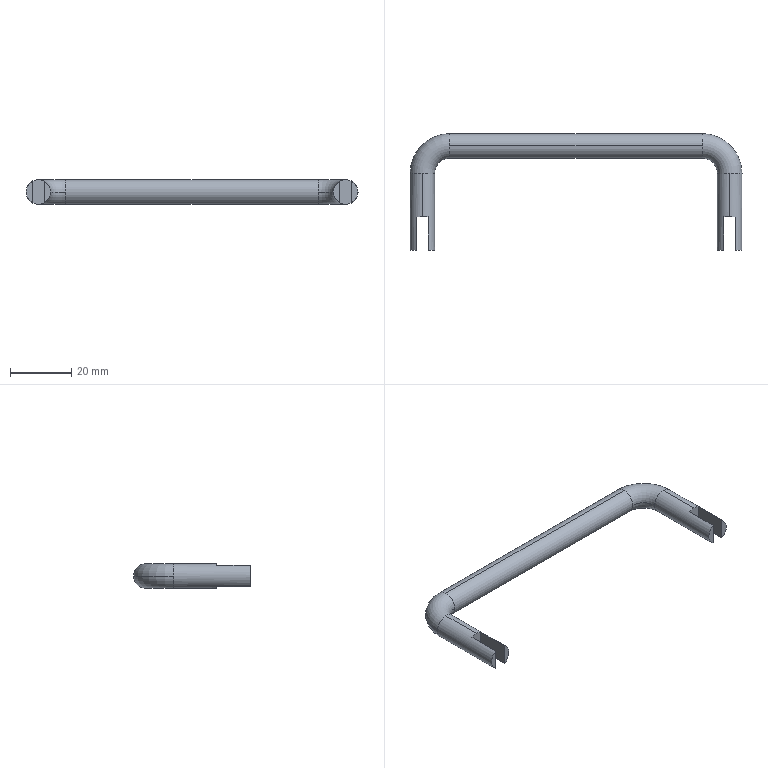Part | STEP file | HI_XAL51-D8-L100-H50-001^XAL51-D8-L100-H50 | 1 solid | 20 faces | box 108 x 38 x 8 mm | volume 7383 mm3 | plane 10 | cylinder 6 | torus 4 | commonest cylinder face diameters 8 x6
STEP:
#1=CARTESIAN_POINT('',(0.,0.,0.));
#2=DIRECTION('',(0.,0.,1.));
#3=DIRECTION('',(1.,0.,0.));
#4=AXIS2_PLACEMENT_3D('',#1,#2,#3);
#5=CARTESIAN_POINT('',(-41.,0.,4.));
#6=VERTEX_POINT('',#5);
#7=CARTESIAN_POINT('',(-41.,4.,0.));
#8=VERTEX_POINT('',#7);
#9=CARTESIAN_POINT('',(-41.,0.,0.));
#10=DIRECTION('',(-1.,0.,0.));
#11=DIRECTION('',(0.,0.,1.));
#12=AXIS2_PLACEMENT_3D('',#9,#10,#11);
#13=CIRCLE('',#12,4.);
#14=CARTESIAN_POINT('',(-41.,-9.,0.));
#15=DIRECTION('',(0.,0.,1.));
#16=DIRECTION('',(1.,0.,0.));
#17=AXIS2_PLACEMENT_3D('',#14,#15,#16);
#18=TOROIDAL_SURFACE('',#17,9.,4.);
#19=CARTESIAN_POINT('',(1.571,1.571));
#20=DIRECTION('',(0.,-1.));
#21=VECTOR('',#20,1.);
#22=LINE('',#19,#21);
#23=(GEOMETRIC_REPRESENTATION_CONTEXT(2)PARAMETRIC_REPRESENTATION_CONTEXT()REPRESENTATION_CONTEXT('',''));
#24=DEFINITIONAL_REPRESENTATION('',(#22),#23);
#25=PCURVE('',#18,#24);
#26=CARTESIAN_POINT('',(41.,0.,0.));
#27=DIRECTION('',(1.,0.,0.));
#28=DIRECTION('',(0.,0.,1.));
#29=AXIS2_PLACEMENT_3D('',#26,#27,#28);
#30=CYLINDRICAL_SURFACE('',#29,4.);
#31=CARTESIAN_POINT('',(6.283,-82.));
#32=DIRECTION('',(-1.,0.));
#33=VECTOR('',#32,1.);
#34=LINE('',#31,#33);
#35=(GEOMETRIC_REPRESENTATION_CONTEXT(2)PARAMETRIC_REPRESENTATION_CONTEXT()REPRESENTATION_CONTEXT('',''));
#36=DEFINITIONAL_REPRESENTATION('',(#34),#35);
#37=PCURVE('',#30,#36);
#38=SURFACE_CURVE('',#13,(#25,#37),.PCURVE_S1.);
#39=EDGE_CURVE('',#6,#8,#38,.T.);
#40=ORIENTED_EDGE('',*,*,#39,.T.);
#41=CARTESIAN_POINT('',(-54.,-9.,0.));
#42=VERTEX_POINT('',#41);
#43=CARTESIAN_POINT('',(-41.,-9.,0.));
#44=DIRECTION('',(0.,0.,1.));
#45=DIRECTION('',(1.,0.,0.));
#46=AXIS2_PLACEMENT_3D('',#43,#44,#45);
#47=CIRCLE('',#46,13.);
#48=CARTESIAN_POINT('',(0.,0.));
#49=DIRECTION('',(1.,0.));
#50=VECTOR('',#49,1.);
#51=LINE('',#48,#50);
#52=(GEOMETRIC_REPRESENTATION_CONTEXT(2)PARAMETRIC_REPRESENTATION_CONTEXT()REPRESENTATION_CONTEXT('',''));
#53=DEFINITIONAL_REPRESENTATION('',(#51),#52);
#54=PCURVE('',#18,#53);
#55=CARTESIAN_POINT('',(-41.,-9.,0.));
#56=DIRECTION('',(0.,0.,1.));
#57=DIRECTION('',(1.,0.,0.));
#58=AXIS2_PLACEMENT_3D('',#55,#56,#57);
#59=TOROIDAL_SURFACE('',#58,9.,4.);
#60=CARTESIAN_POINT('',(0.,6.283));
#61=DIRECTION('',(1.,0.));
#62=VECTOR('',#61,1.);
#63=LINE('',#60,#62);
#64=(GEOMETRIC_REPRESENTATION_CONTEXT(2)PARAMETRIC_REPRESENTATION_CONTEXT()REPRESENTATION_CONTEXT('',''));
#65=DEFINITIONAL_REPRESENTATION('',(#63),#64);
#66=PCURVE('',#59,#65);
#67=SURFACE_CURVE('',#47,(#54,#66),.PCURVE_S1.);
#68=EDGE_CURVE('',#8,#42,#67,.T.);
#69=ORIENTED_EDGE('',*,*,#68,.T.);
#70=CARTESIAN_POINT('',(-50.,-9.,4.));
#71=VERTEX_POINT('',#70);
#72=CARTESIAN_POINT('',(-50.,-9.,0.));
#73=DIRECTION('',(0.,-1.,0.));
#74=DIRECTION('',(0.,0.,1.));
#75=AXIS2_PLACEMENT_3D('',#72,#73,#74);
#76=CIRCLE('',#75,4.);
#77=CARTESIAN_POINT('',(3.142,1.571));
#78=DIRECTION('',(0.,-1.));
#79=VECTOR('',#78,1.);
#80=LINE('',#77,#79);
#81=(GEOMETRIC_REPRESENTATION_CONTEXT(2)PARAMETRIC_REPRESENTATION_CONTEXT()REPRESENTATION_CONTEXT('',''));
#82=DEFINITIONAL_REPRESENTATION('',(#80),#81);
#83=PCURVE('',#18,#82);
#84=CARTESIAN_POINT('',(-50.,-34.,0.));
#85=DIRECTION('',(0.,-1.,0.));
#86=DIRECTION('',(0.,0.,1.));
#87=AXIS2_PLACEMENT_3D('',#84,#85,#86);
#88=CYLINDRICAL_SURFACE('',#87,4.);
#89=CARTESIAN_POINT('',(0.,-25.));
#90=DIRECTION('',(1.,0.));
#91=VECTOR('',#90,1.);
#92=LINE('',#89,#91);
#93=(GEOMETRIC_REPRESENTATION_CONTEXT(2)PARAMETRIC_REPRESENTATION_CONTEXT()REPRESENTATION_CONTEXT('',''));
#94=DEFINITIONAL_REPRESENTATION('',(#92),#93);
#95=PCURVE('',#88,#94);
#96=SURFACE_CURVE('',#76,(#83,#95),.PCURVE_S1.);
#97=EDGE_CURVE('',#71,#42,#96,.T.);
#98=ORIENTED_EDGE('',*,*,#97,.F.);
#99=CARTESIAN_POINT('',(-46.,-9.,0.));
#100=VERTEX_POINT('',#99);
#101=CARTESIAN_POINT('',(-50.,-9.,0.));
#102=DIRECTION('',(0.,-1.,0.));
#103=DIRECTION('',(0.,0.,1.));
#104=AXIS2_PLACEMENT_3D('',#101,#102,#103);
#105=CIRCLE('',#104,4.);
#106=CARTESIAN_POINT('',(3.142,7.854));
#107=DIRECTION('',(0.,-1.));
#108=VECTOR('',#107,1.);
#109=LINE('',#106,#108);
#110=(GEOMETRIC_REPRESENTATION_CONTEXT(2)PARAMETRIC_REPRESENTATION_CONTEXT()REPRESENTATION_CONTEXT('',''));
#111=DEFINITIONAL_REPRESENTATION('',(#109),#110);
#112=PCURVE('',#18,#111);
#113=CARTESIAN_POINT('',(-50.,-34.,0.));
#114=DIRECTION('',(0.,-1.,0.));
#115=DIRECTION('',(0.,0.,1.));
#116=AXIS2_PLACEMENT_3D('',#113,#114,#115);
#117=CYLINDRICAL_SURFACE('',#116,4.);
#118=CARTESIAN_POINT('',(0.,-25.));
#119=DIRECTION('',(1.,0.));
#120=VECTOR('',#119,1.);
#121=LINE('',#118,#120);
#122=(GEOMETRIC_REPRESENTATION_CONTEXT(2)PARAMETRIC_REPRESENTATION_CONTEXT()REPRESENTATION_CONTEXT('',''));
#123=DEFINITIONAL_REPRESENTATION('',(#121),#122);
#124=PCURVE('',#117,#123);
#125=SURFACE_CURVE('',#105,(#112,#124),.PCURVE_S1.);
#126=EDGE_CURVE('',#100,#71,#125,.T.);
#127=ORIENTED_EDGE('',*,*,#126,.F.);
#128=CARTESIAN_POINT('',(-41.,-4.,0.));
#129=VERTEX_POINT('',#128);
#130=CARTESIAN_POINT('',(-41.,-9.,0.));
#131=DIRECTION('',(0.,0.,1.));
#132=DIRECTION('',(1.,0.,0.));
#133=AXIS2_PLACEMENT_3D('',#130,#131,#132);
#134=CIRCLE('',#133,5.);
#135=CARTESIAN_POINT('',(0.,3.142));
#136=DIRECTION('',(1.,0.));
#137=VECTOR('',#136,1.);
#138=LINE('',#135,#137);
#139=(GEOMETRIC_REPRESENTATION_CONTEXT(2)PARAMETRIC_REPRESENTATION_CONTEXT()REPRESENTATION_CONTEXT('',''));
#140=DEFINITIONAL_REPRESENTATION('',(#138),#139);
#141=PCURVE('',#18,#140);
#142=CARTESIAN_POINT('',(0.,3.142));
#143=DIRECTION('',(1.,0.));
#144=VECTOR('',#143,1.);
#145=LINE('',#142,#144);
#146=(GEOMETRIC_REPRESENTATION_CONTEXT(2)PARAMETRIC_REPRESENTATION_CONTEXT()REPRESENTATION_CONTEXT('',''));
#147=DEFINITIONAL_REPRESENTATION('',(#145),#146);
#148=PCURVE('',#59,#147);
#149=SURFACE_CURVE('',#134,(#141,#148),.PCURVE_S1.);
#150=EDGE_CURVE('',#129,#100,#149,.T.);
#151=ORIENTED_EDGE('',*,*,#150,.F.);
#152=CARTESIAN_POINT('',(-41.,0.,0.));
#153=DIRECTION('',(-1.,0.,0.));
#154=DIRECTION('',(0.,0.,1.));
#155=AXIS2_PLACEMENT_3D('',#152,#153,#154);
#156=CIRCLE('',#155,4.);
#157=CARTESIAN_POINT('',(1.571,7.854));
#158=DIRECTION('',(0.,-1.));
#159=VECTOR('',#158,1.);
#160=LINE('',#157,#159);
#161=(GEOMETRIC_REPRESENTATION_CONTEXT(2)PARAMETRIC_REPRESENTATION_CONTEXT()REPRESENTATION_CONTEXT('',''));
#162=DEFINITIONAL_REPRESENTATION('',(#160),#161);
#163=PCURVE('',#18,#162);
#164=CARTESIAN_POINT('',(41.,0.,0.));
#165=DIRECTION('',(1.,0.,0.));
#166=DIRECTION('',(0.,0.,1.));
#167=AXIS2_PLACEMENT_3D('',#164,#165,#166);
#168=CYLINDRICAL_SURFACE('',#167,4.);
#169=CARTESIAN_POINT('',(6.283,-82.));
#170=DIRECTION('',(-1.,0.));
#171=VECTOR('',#170,1.);
#172=LINE('',#169,#171);
#173=(GEOMETRIC_REPRESENTATION_CONTEXT(2)PARAMETRIC_REPRESENTATION_CONTEXT()REPRESENTATION_CONTEXT('',''));
#174=DEFINITIONAL_REPRESENTATION('',(#172),#173);
#175=PCURVE('',#168,#174);
#176=SURFACE_CURVE('',#156,(#163,#175),.PCURVE_S1.);
#177=EDGE_CURVE('',#129,#6,#176,.T.);
#178=ORIENTED_EDGE('',*,*,#177,.T.);
#179=EDGE_LOOP('',(#40,#69,#98,#127,#151,#178));
#180=FACE_BOUND('',#179,.T.);
#181=ADVANCED_FACE('',(#180),#18,.T.);
#182=CARTESIAN_POINT('',(41.,0.,-4.));
#183=VERTEX_POINT('',#182);
#184=CARTESIAN_POINT('',(41.,4.,0.));
#185=VERTEX_POINT('',#184);
#186=CARTESIAN_POINT('',(41.,0.,0.));
#187=DIRECTION('',(1.,0.,0.));
#188=DIRECTION('',(0.,0.,-1.));
#189=AXIS2_PLACEMENT_3D('',#186,#187,#188);
#190=CIRCLE('',#189,4.);
#191=CARTESIAN_POINT('',(41.,-9.,0.));
#192=DIRECTION('',(0.,0.,-1.));
#193=DIRECTION('',(-1.,0.,0.));
#194=AXIS2_PLACEMENT_3D('',#191,#192,#193);
#195=TOROIDAL_SURFACE('',#194,9.,4.);
#196=CARTESIAN_POINT('',(1.571,1.571));
#197=DIRECTION('',(0.,-1.));
#198=VECTOR('',#197,1.);
#199=LINE('',#196,#198);
#200=(GEOMETRIC_REPRESENTATION_CONTEXT(2)PARAMETRIC_REPRESENTATION_CONTEXT()REPRESENTATION_CONTEXT('',''));
#201=DEFINITIONAL_REPRESENTATION('',(#199),#200);
#202=PCURVE('',#195,#201);
#203=CARTESIAN_POINT('',(3.142,0.));
#204=DIRECTION('',(1.,0.));
#205=VECTOR('',#204,1.);
#206=LINE('',#203,#205);
#207=(GEOMETRIC_REPRESENTATION_CONTEXT(2)PARAMETRIC_REPRESENTATION_CONTEXT()REPRESENTATION_CONTEXT('',''));
#208=DEFINITIONAL_REPRESENTATION('',(#206),#207);
#209=PCURVE('',#30,#208);
#210=SURFACE_CURVE('',#190,(#202,#209),.PCURVE_S1.);
#211=EDGE_CURVE('',#183,#185,#210,.T.);
#212=ORIENTED_EDGE('',*,*,#211,.T.);
#213=CARTESIAN_POINT('',(54.,-9.,0.));
#214=VERTEX_POINT('',#213);
#215=CARTESIAN_POINT('',(41.,-9.,0.));
#216=DIRECTION('',(0.,0.,-1.));
#217=DIRECTION('',(-1.,0.,0.));
#218=AXIS2_PLACEMENT_3D('',#215,#216,#217);
#219=CIRCLE('',#218,13.);
#220=CARTESIAN_POINT('',(0.,0.));
#221=DIRECTION('',(1.,0.));
#222=VECTOR('',#221,1.);
#223=LINE('',#220,#222);
#224=(GEOMETRIC_REPRESENTATION_CONTEXT(2)PARAMETRIC_REPRESENTATION_CONTEXT()REPRESENTATION_CONTEXT('',''));
#225=DEFINITIONAL_REPRESENTATION('',(#223),#224);
#226=PCURVE('',#195,#225);
#227=CARTESIAN_POINT('',(41.,-9.,0.));
#228=DIRECTION('',(0.,0.,-1.));
#229=DIRECTION('',(-1.,0.,0.));
#230=AXIS2_PLACEMENT_3D('',#227,#228,#229);
#231=TOROIDAL_SURFACE('',#230,9.,4.);
#232=CARTESIAN_POINT('',(0.,6.283));
#233=DIRECTION('',(1.,0.));
#234=VECTOR('',#233,1.);
#235=LINE('',#232,#234);
#236=(GEOMETRIC_REPRESENTATION_CONTEXT(2)PARAMETRIC_REPRESENTATION_CONTEXT()REPRESENTATION_CONTEXT('',''));
#237=DEFINITIONAL_REPRESENTATION('',(#235),#236);
#238=PCURVE('',#231,#237);
#239=SURFACE_CURVE('',#219,(#226,#238),.PCURVE_S1.);
#240=EDGE_CURVE('',#185,#214,#239,.T.);
#241=ORIENTED_EDGE('',*,*,#240,.T.);
#242=CARTESIAN_POINT('',(50.,-9.,-4.));
#243=VERTEX_POINT('',#242);
#244=CARTESIAN_POINT('',(50.,-9.,0.));
#245=DIRECTION('',(0.,-1.,0.));
#246=DIRECTION('',(0.,0.,-1.));
#247=AXIS2_PLACEMENT_3D('',#244,#245,#246);
#248=CIRCLE('',#247,4.);
#249=CARTESIAN_POINT('',(3.142,1.571));
#250=DIRECTION('',(0.,-1.));
#251=VECTOR('',#250,1.);
#252=LINE('',#249,#251);
#253=(GEOMETRIC_REPRESENTATION_CONTEXT(2)PARAMETRIC_REPRESENTATION_CONTEXT()REPRESENTATION_CONTEXT('',''));
#254=DEFINITIONAL_REPRESENTATION('',(#252),#253);
#255=PCURVE('',#195,#254);
#256=CARTESIAN_POINT('',(50.,-34.,0.));
#257=DIRECTION('',(0.,-1.,0.));
#258=DIRECTION('',(0.,0.,1.));
#259=AXIS2_PLACEMENT_3D('',#256,#257,#258);
#260=CYLINDRICAL_SURFACE('',#259,4.);
#261=CARTESIAN_POINT('',(3.142,-25.));
#262=DIRECTION('',(1.,0.));
#263=VECTOR('',#262,1.);
#264=LINE('',#261,#263);
#265=(GEOMETRIC_REPRESENTATION_CONTEXT(2)PARAMETRIC_REPRESENTATION_CONTEXT()REPRESENTATION_CONTEXT('',''));
#266=DEFINITIONAL_REPRESENTATION('',(#264),#265);
#267=PCURVE('',#260,#266);
#268=SURFACE_CURVE('',#248,(#255,#267),.PCURVE_S1.);
#269=EDGE_CURVE('',#243,#214,#268,.T.);
#270=ORIENTED_EDGE('',*,*,#269,.F.);
#271=CARTESIAN_POINT('',(46.,-9.,0.));
#272=VERTEX_POINT('',#271);
#273=CARTESIAN_POINT('',(50.,-9.,0.));
#274=DIRECTION('',(0.,-1.,0.));
#275=DIRECTION('',(0.,0.,-1.));
#276=AXIS2_PLACEMENT_3D('',#273,#274,#275);
#277=CIRCLE('',#276,4.);
#278=CARTESIAN_POINT('',(3.142,7.854));
#279=DIRECTION('',(0.,-1.));
#280=VECTOR('',#279,1.);
#281=LINE('',#278,#280);
#282=(GEOMETRIC_REPRESENTATION_CONTEXT(2)PARAMETRIC_REPRESENTATION_CONTEXT()REPRESENTATION_CONTEXT('',''));
#283=DEFINITIONAL_REPRESENTATION('',(#281),#282);
#284=PCURVE('',#195,#283);
#285=CARTESIAN_POINT('',(50.,-34.,0.));
#286=DIRECTION('',(0.,-1.,0.));
#287=DIRECTION('',(0.,0.,1.));
#288=AXIS2_PLACEMENT_3D('',#285,#286,#287);
#289=CYLINDRICAL_SURFACE('',#288,4.);
#290=CARTESIAN_POINT('',(-3.142,-25.));
#291=DIRECTION('',(1.,0.));
#292=VECTOR('',#291,1.);
#293=LINE('',#290,#292);
#294=(GEOMETRIC_REPRESENTATION_CONTEXT(2)PARAMETRIC_REPRESENTATION_CONTEXT()REPRESENTATION_CONTEXT('',''));
#295=DEFINITIONAL_REPRESENTATION('',(#293),#294);
#296=PCURVE('',#289,#295);
#297=SURFACE_CURVE('',#277,(#284,#296),.PCURVE_S1.);
#298=EDGE_CURVE('',#272,#243,#297,.T.);
#299=ORIENTED_EDGE('',*,*,#298,.F.);
#300=CARTESIAN_POINT('',(41.,-4.,0.));
#301=VERTEX_POINT('',#300);
#302=CARTESIAN_POINT('',(41.,-9.,0.));
#303=DIRECTION('',(0.,0.,-1.));
#304=DIRECTION('',(-1.,0.,0.));
#305=AXIS2_PLACEMENT_3D('',#302,#303,#304);
#306=CIRCLE('',#305,5.);
#307=CARTESIAN_POINT('',(0.,3.142));
#308=DIRECTION('',(1.,0.));
#309=VECTOR('',#308,1.);
#310=LINE('',#307,#309);
#311=(GEOMETRIC_REPRESENTATION_CONTEXT(2)PARAMETRIC_REPRESENTATION_CONTEXT()REPRESENTATION_CONTEXT('',''));
#312=DEFINITIONAL_REPRESENTATION('',(#310),#311);
#313=PCURVE('',#195,#312);
#314=CARTESIAN_POINT('',(0.,3.142));
#315=DIRECTION('',(1.,0.));
#316=VECTOR('',#315,1.);
#317=LINE('',#314,#316);
#318=(GEOMETRIC_REPRESENTATION_CONTEXT(2)PARAMETRIC_REPRESENTATION_CONTEXT()REPRESENTATION_CONTEXT('',''));
#319=DEFINITIONAL_REPRESENTATION('',(#317),#318);
#320=PCURVE('',#231,#319);
#321=SURFACE_CURVE('',#306,(#313,#320),.PCURVE_S1.);
#322=EDGE_CURVE('',#301,#272,#321,.T.);
#323=ORIENTED_EDGE('',*,*,#322,.F.);
#324=CARTESIAN_POINT('',(41.,0.,0.));
#325=DIRECTION('',(1.,0.,0.));
#326=DIRECTION('',(0.,0.,-1.));
#327=AXIS2_PLACEMENT_3D('',#324,#325,#326);
#328=CIRCLE('',#327,4.);
#329=CARTESIAN_POINT('',(1.571,7.854));
#330=DIRECTION('',(0.,-1.));
#331=VECTOR('',#330,1.);
#332=LINE('',#329,#331);
#333=(GEOMETRIC_REPRESENTATION_CONTEXT(2)PARAMETRIC_REPRESENTATION_CONTEXT()REPRESENTATION_CONTEXT('',''));
#334=DEFINITIONAL_REPRESENTATION('',(#332),#333);
#335=PCURVE('',#195,#334);
#336=CARTESIAN_POINT('',(-3.142,0.));
#337=DIRECTION('',(1.,0.));
#338=VECTOR('',#337,1.);
#339=LINE('',#336,#338);
#340=(GEOMETRIC_REPRESENTATION_CONTEXT(2)PARAMETRIC_REPRESENTATION_CONTEXT()REPRESENTATION_CONTEXT('',''));
#341=DEFINITIONAL_REPRESENTATION('',(#339),#340);
#342=PCURVE('',#168,#341);
#343=SURFACE_CURVE('',#328,(#335,#342),.PCURVE_S1.);
#344=EDGE_CURVE('',#301,#183,#343,.T.);
#345=ORIENTED_EDGE('',*,*,#344,.T.);
#346=EDGE_LOOP('',(#212,#241,#270,#299,#323,#345));
#347=FACE_BOUND('',#346,.T.);
#348=ADVANCED_FACE('',(#347),#195,.T.);
#349=CARTESIAN_POINT('',(50.,-9.,4.));
#350=VERTEX_POINT('',#349);
#351=CARTESIAN_POINT('',(50.,-9.,0.));
#352=DIRECTION('',(0.,-1.,0.));
#353=DIRECTION('',(0.,0.,-1.));
#354=AXIS2_PLACEMENT_3D('',#351,#352,#353);
#355=CIRCLE('',#354,4.);
#356=CARTESIAN_POINT('',(-3.142,-25.));
#357=DIRECTION('',(1.,0.));
#358=VECTOR('',#357,1.);
#359=LINE('',#356,#358);
#360=(GEOMETRIC_REPRESENTATION_CONTEXT(2)PARAMETRIC_REPRESENTATION_CONTEXT()REPRESENTATION_CONTEXT('',''));
#361=DEFINITIONAL_REPRESENTATION('',(#359),#360);
#362=PCURVE('',#289,#361);
#363=CARTESIAN_POINT('',(3.142,7.854));
#364=DIRECTION('',(0.,-1.));
#365=VECTOR('',#364,1.);
#366=LINE('',#363,#365);
#367=(GEOMETRIC_REPRESENTATION_CONTEXT(2)PARAMETRIC_REPRESENTATION_CONTEXT()REPRESENTATION_CONTEXT('',''));
#368=DEFINITIONAL_REPRESENTATION('',(#366),#367);
#369=PCURVE('',#231,#368);
#370=SURFACE_CURVE('',#355,(#362,#369),.PCURVE_S1.);
#371=EDGE_CURVE('',#350,#272,#370,.T.);
#372=ORIENTED_EDGE('',*,*,#371,.T.);
#373=ORIENTED_EDGE('',*,*,#298,.T.);
#374=CARTESIAN_POINT('',(50.,-23.,-4.));
#375=VERTEX_POINT('',#374);
#376=CARTESIAN_POINT('',(50.,-34.,-4.));
#377=DIRECTION('',(0.,-1.,0.));
#378=VECTOR('',#377,1.);
#379=LINE('',#376,#378);
#380=CARTESIAN_POINT('',(3.142,0.));
#381=DIRECTION('',(0.,1.));
#382=VECTOR('',#381,1.);
#383=LINE('',#380,#382);
#384=(GEOMETRIC_REPRESENTATION_CONTEXT(2)PARAMETRIC_REPRESENTATION_CONTEXT()REPRESENTATION_CONTEXT('',''));
#385=DEFINITIONAL_REPRESENTATION('',(#383),#384);
#386=PCURVE('',#289,#385);
#387=CARTESIAN_POINT('',(3.142,0.));
#388=DIRECTION('',(0.,1.));
#389=VECTOR('',#388,1.);
#390=LINE('',#387,#389);
#391=(GEOMETRIC_REPRESENTATION_CONTEXT(2)PARAMETRIC_REPRESENTATION_CONTEXT()REPRESENTATION_CONTEXT('',''));
#392=DEFINITIONAL_REPRESENTATION('',(#390),#391);
#393=PCURVE('',#260,#392);
#394=SURFACE_CURVE('',#379,(#386,#393),.PCURVE_S1.);
#395=EDGE_CURVE('',#243,#375,#394,.T.);
#396=ORIENTED_EDGE('',*,*,#395,.T.);
#397=CARTESIAN_POINT('',(48.,-23.,-3.464));
#398=VERTEX_POINT('',#397);
#399=CARTESIAN_POINT('',(50.,-23.,0.));
#400=DIRECTION('',(0.,-1.,0.));
#401=DIRECTION('',(0.,0.,-1.));
#402=AXIS2_PLACEMENT_3D('',#399,#400,#401);
#403=CIRCLE('',#402,4.);
#404=CARTESIAN_POINT('',(-3.142,-11.));
#405=DIRECTION('',(1.,0.));
#406=VECTOR('',#405,1.);
#407=LINE('',#404,#406);
#408=(GEOMETRIC_REPRESENTATION_CONTEXT(2)PARAMETRIC_REPRESENTATION_CONTEXT()REPRESENTATION_CONTEXT('',''));
#409=DEFINITIONAL_REPRESENTATION('',(#407),#408);
#410=PCURVE('',#289,#409);
#411=CARTESIAN_POINT('',(52.,-23.,16.));
#412=DIRECTION('',(0.,-1.,0.));
#413=DIRECTION('',(0.,0.,-1.));
#414=AXIS2_PLACEMENT_3D('',#411,#412,#413);
#415=PLANE('',#414);
#416=CARTESIAN_POINT('',(16.,-2.));
#417=DIRECTION('',(1.,0.));
#418=AXIS2_PLACEMENT_2D('',#416,#417);
#419=CIRCLE('',#418,4.);
#420=(GEOMETRIC_REPRESENTATION_CONTEXT(2)PARAMETRIC_REPRESENTATION_CONTEXT()REPRESENTATION_CONTEXT('',''));
#421=DEFINITIONAL_REPRESENTATION('',(#419),#420);
#422=PCURVE('',#415,#421);
#423=SURFACE_CURVE('',#403,(#410,#422),.PCURVE_S1.);
#424=EDGE_CURVE('',#398,#375,#423,.T.);
#425=ORIENTED_EDGE('',*,*,#424,.F.);
#426=CARTESIAN_POINT('',(48.,-34.,-3.464));
#427=VERTEX_POINT('',#426);
#428=CARTESIAN_POINT('',(48.,-34.,-3.464));
#429=DIRECTION('',(0.,1.,0.));
#430=VECTOR('',#429,1.);
#431=LINE('',#428,#430);
#432=CARTESIAN_POINT('',(2.618,0.));
#433=DIRECTION('',(0.,-1.));
#434=VECTOR('',#433,1.);
#435=LINE('',#432,#434);
#436=(GEOMETRIC_REPRESENTATION_CONTEXT(2)PARAMETRIC_REPRESENTATION_CONTEXT()REPRESENTATION_CONTEXT('',''));
#437=DEFINITIONAL_REPRESENTATION('',(#435),#436);
#438=PCURVE('',#289,#437);
#439=CARTESIAN_POINT('',(48.,-23.,16.));
#440=DIRECTION('',(1.,0.,0.));
#441=DIRECTION('',(0.,1.,0.));
#442=AXIS2_PLACEMENT_3D('',#439,#440,#441);
#443=PLANE('',#442);
#444=CARTESIAN_POINT('',(-11.,-19.464));
#445=DIRECTION('',(1.,0.));
#446=VECTOR('',#445,1.);
#447=LINE('',#444,#446);
#448=(GEOMETRIC_REPRESENTATION_CONTEXT(2)PARAMETRIC_REPRESENTATION_CONTEXT()REPRESENTATION_CONTEXT('',''));
#449=DEFINITIONAL_REPRESENTATION('',(#447),#448);
#450=PCURVE('',#443,#449);
#451=SURFACE_CURVE('',#431,(#438,#450),.PCURVE_S1.);
#452=EDGE_CURVE('',#427,#398,#451,.T.);
#453=ORIENTED_EDGE('',*,*,#452,.F.);
#454=CARTESIAN_POINT('',(48.,-34.,3.464));
#455=VERTEX_POINT('',#454);
#456=CARTESIAN_POINT('',(50.,-34.,0.));
#457=DIRECTION('',(0.,-1.,0.));
#458=DIRECTION('',(0.,0.,-1.));
#459=AXIS2_PLACEMENT_3D('',#456,#457,#458);
#460=CIRCLE('',#459,4.);
#461=CARTESIAN_POINT('',(-3.142,0.));
#462=DIRECTION('',(1.,0.));
#463=VECTOR('',#462,1.);
#464=LINE('',#461,#463);
#465=(GEOMETRIC_REPRESENTATION_CONTEXT(2)PARAMETRIC_REPRESENTATION_CONTEXT()REPRESENTATION_CONTEXT('',''));
#466=DEFINITIONAL_REPRESENTATION('',(#464),#465);
#467=PCURVE('',#289,#466);
#468=CARTESIAN_POINT('',(50.,-34.,0.));
#469=DIRECTION('',(0.,-1.,0.));
#470=DIRECTION('',(0.,0.,-1.));
#471=AXIS2_PLACEMENT_3D('',#468,#469,#470);
#472=PLANE('',#471);
#473=CARTESIAN_POINT('',(0.,0.));
#474=DIRECTION('',(1.,0.));
#475=AXIS2_PLACEMENT_2D('',#473,#474);
#476=CIRCLE('',#475,4.);
#477=(GEOMETRIC_REPRESENTATION_CONTEXT(2)PARAMETRIC_REPRESENTATION_CONTEXT()REPRESENTATION_CONTEXT('',''));
#478=DEFINITIONAL_REPRESENTATION('',(#476),#477);
#479=PCURVE('',#472,#478);
#480=SURFACE_CURVE('',#460,(#467,#479),.PCURVE_S1.);
#481=EDGE_CURVE('',#455,#427,#480,.T.);
#482=ORIENTED_EDGE('',*,*,#481,.F.);
#483=CARTESIAN_POINT('',(48.,-23.,3.464));
#484=VERTEX_POINT('',#483);
#485=CARTESIAN_POINT('',(48.,-34.,3.464));
#486=DIRECTION('',(0.,-1.,0.));
#487=VECTOR('',#486,1.);
#488=LINE('',#485,#487);
#489=CARTESIAN_POINT('',(0.5236,0.));
#490=DIRECTION('',(0.,1.));
#491=VECTOR('',#490,1.);
#492=LINE('',#489,#491);
#493=(GEOMETRIC_REPRESENTATION_CONTEXT(2)PARAMETRIC_REPRESENTATION_CONTEXT()REPRESENTATION_CONTEXT('',''));
#494=DEFINITIONAL_REPRESENTATION('',(#492),#493);
#495=PCURVE('',#289,#494);
#496=CARTESIAN_POINT('',(-11.,-12.536));
#497=DIRECTION('',(-1.,0.));
#498=VECTOR('',#497,1.);
#499=LINE('',#496,#498);
#500=(GEOMETRIC_REPRESENTATION_CONTEXT(2)PARAMETRIC_REPRESENTATION_CONTEXT()REPRESENTATION_CONTEXT('',''));
#501=DEFINITIONAL_REPRESENTATION('',(#499),#500);
#502=PCURVE('',#443,#501);
#503=SURFACE_CURVE('',#488,(#495,#502),.PCURVE_S1.);
#504=EDGE_CURVE('',#484,#455,#503,.T.);
#505=ORIENTED_EDGE('',*,*,#504,.F.);
#506=CARTESIAN_POINT('',(50.,-23.,4.));
#507=VERTEX_POINT('',#506);
#508=CARTESIAN_POINT('',(50.,-23.,0.));
#509=DIRECTION('',(0.,-1.,0.));
#510=DIRECTION('',(0.,0.,-1.));
#511=AXIS2_PLACEMENT_3D('',#508,#509,#510);
#512=CIRCLE('',#511,4.);
#513=CARTESIAN_POINT('',(-3.142,-11.));
#514=DIRECTION('',(1.,0.));
#515=VECTOR('',#514,1.);
#516=LINE('',#513,#515);
#517=(GEOMETRIC_REPRESENTATION_CONTEXT(2)PARAMETRIC_REPRESENTATION_CONTEXT()REPRESENTATION_CONTEXT('',''));
#518=DEFINITIONAL_REPRESENTATION('',(#516),#517);
#519=PCURVE('',#289,#518);
#520=CARTESIAN_POINT('',(16.,-2.));
#521=DIRECTION('',(1.,0.));
#522=AXIS2_PLACEMENT_2D('',#520,#521);
#523=CIRCLE('',#522,4.);
#524=(GEOMETRIC_REPRESENTATION_CONTEXT(2)PARAMETRIC_REPRESENTATION_CONTEXT()REPRESENTATION_CONTEXT('',''));
#525=DEFINITIONAL_REPRESENTATION('',(#523),#524);
#526=PCURVE('',#415,#525);
#527=SURFACE_CURVE('',#512,(#519,#526),.PCURVE_S1.);
#528=EDGE_CURVE('',#507,#484,#527,.T.);
#529=ORIENTED_EDGE('',*,*,#528,.F.);
#530=CARTESIAN_POINT('',(50.,-34.,4.));
#531=DIRECTION('',(0.,-1.,0.));
#532=VECTOR('',#531,1.);
#533=LINE('',#530,#532);
#534=CARTESIAN_POINT('',(0.,0.));
#535=DIRECTION('',(0.,1.));
#536=VECTOR('',#535,1.);
#537=LINE('',#534,#536);
#538=(GEOMETRIC_REPRESENTATION_CONTEXT(2)PARAMETRIC_REPRESENTATION_CONTEXT()REPRESENTATION_CONTEXT('',''));
#539=DEFINITIONAL_REPRESENTATION('',(#537),#538);
#540=PCURVE('',#289,#539);
#541=CARTESIAN_POINT('',(6.283,0.));
#542=DIRECTION('',(0.,1.));
#543=VECTOR('',#542,1.);
#544=LINE('',#541,#543);
#545=(GEOMETRIC_REPRESENTATION_CONTEXT(2)PARAMETRIC_REPRESENTATION_CONTEXT()REPRESENTATION_CONTEXT('',''));
#546=DEFINITIONAL_REPRESENTATION('',(#544),#545);
#547=PCURVE('',#260,#546);
#548=SURFACE_CURVE('',#533,(#540,#547),.PCURVE_S1.);
#549=EDGE_CURVE('',#350,#507,#548,.T.);
#550=ORIENTED_EDGE('',*,*,#549,.F.);
#551=EDGE_LOOP('',(#372,#373,#396,#425,#453,#482,#505,#529,#550));
#552=FACE_BOUND('',#551,.T.);
#553=ADVANCED_FACE('',(#552),#289,.T.);
#554=CARTESIAN_POINT('',(-41.,0.,-4.));
#555=VERTEX_POINT('',#554);
#556=CARTESIAN_POINT('',(-41.,0.,0.));
#557=DIRECTION('',(-1.,0.,0.));
#558=DIRECTION('',(0.,0.,1.));
#559=AXIS2_PLACEMENT_3D('',#556,#557,#558);
#560=CIRCLE('',#559,4.);
#561=CARTESIAN_POINT('',(6.283,-82.));
#562=DIRECTION('',(-1.,0.));
#563=VECTOR('',#562,1.);
#564=LINE('',#561,#563);
#565=(GEOMETRIC_REPRESENTATION_CONTEXT(2)PARAMETRIC_REPRESENTATION_CONTEXT()REPRESENTATION_CONTEXT('',''));
#566=DEFINITIONAL_REPRESENTATION('',(#564),#565);
#567=PCURVE('',#168,#566);
#568=CARTESIAN_POINT('',(1.571,7.854));
#569=DIRECTION('',(0.,-1.));
#570=VECTOR('',#569,1.);
#571=LINE('',#568,#570);
#572=(GEOMETRIC_REPRESENTATION_CONTEXT(2)PARAMETRIC_REPRESENTATION_CONTEXT()REPRESENTATION_CONTEXT('',''));
#573=DEFINITIONAL_REPRESENTATION('',(#571),#572);
#574=PCURVE('',#59,#573);
#575=SURFACE_CURVE('',#560,(#567,#574),.PCURVE_S1.);
#576=EDGE_CURVE('',#555,#129,#575,.T.);
#577=ORIENTED_EDGE('',*,*,#576,.F.);
#578=CARTESIAN_POINT('',(41.,0.,-4.));
#579=DIRECTION('',(1.,0.,0.));
#580=VECTOR('',#579,1.);
#581=LINE('',#578,#580);
#582=CARTESIAN_POINT('',(3.142,0.));
#583=DIRECTION('',(0.,1.));
#584=VECTOR('',#583,1.);
#585=LINE('',#582,#584);
#586=(GEOMETRIC_REPRESENTATION_CONTEXT(2)PARAMETRIC_REPRESENTATION_CONTEXT()REPRESENTATION_CONTEXT('',''));
#587=DEFINITIONAL_REPRESENTATION('',(#585),#586);
#588=PCURVE('',#168,#587);
#589=CARTESIAN_POINT('',(3.142,0.));
#590=DIRECTION('',(0.,1.));
#591=VECTOR('',#590,1.);
#592=LINE('',#589,#591);
#593=(GEOMETRIC_REPRESENTATION_CONTEXT(2)PARAMETRIC_REPRESENTATION_CONTEXT()REPRESENTATION_CONTEXT('',''));
#594=DEFINITIONAL_REPRESENTATION('',(#592),#593);
#595=PCURVE('',#30,#594);
#596=SURFACE_CURVE('',#581,(#588,#595),.PCURVE_S1.);
#597=EDGE_CURVE('',#555,#183,#596,.T.);
#598=ORIENTED_EDGE('',*,*,#597,.T.);
#599=ORIENTED_EDGE('',*,*,#344,.F.);
#600=CARTESIAN_POINT('',(41.,0.,4.));
#601=VERTEX_POINT('',#600);
#602=CARTESIAN_POINT('',(41.,0.,0.));
#603=DIRECTION('',(1.,0.,0.));
#604=DIRECTION('',(0.,0.,-1.));
#605=AXIS2_PLACEMENT_3D('',#602,#603,#604);
#606=CIRCLE('',#605,4.);
#607=CARTESIAN_POINT('',(-3.142,0.));
#608=DIRECTION('',(1.,0.));
#609=VECTOR('',#608,1.);
#610=LINE('',#607,#609);
#611=(GEOMETRIC_REPRESENTATION_CONTEXT(2)PARAMETRIC_REPRESENTATION_CONTEXT()REPRESENTATION_CONTEXT('',''));
#612=DEFINITIONAL_REPRESENTATION('',(#610),#611);
#613=PCURVE('',#168,#612);
#614=CARTESIAN_POINT('',(1.571,7.854));
#615=DIRECTION('',(0.,-1.));
#616=VECTOR('',#615,1.);
#617=LINE('',#614,#616);
#618=(GEOMETRIC_REPRESENTATION_CONTEXT(2)PARAMETRIC_REPRESENTATION_CONTEXT()REPRESENTATION_CONTEXT('',''));
#619=DEFINITIONAL_REPRESENTATION('',(#617),#618);
#620=PCURVE('',#231,#619);
#621=SURFACE_CURVE('',#606,(#613,#620),.PCURVE_S1.);
#622=EDGE_CURVE('',#601,#301,#621,.T.);
#623=ORIENTED_EDGE('',*,*,#622,.F.);
#624=CARTESIAN_POINT('',(41.,0.,4.));
#625=DIRECTION('',(1.,0.,0.));
#626=VECTOR('',#625,1.);
#627=LINE('',#624,#626);
#628=CARTESIAN_POINT('',(0.,0.));
#629=DIRECTION('',(0.,1.));
#630=VECTOR('',#629,1.);
#631=LINE('',#628,#630);
#632=(GEOMETRIC_REPRESENTATION_CONTEXT(2)PARAMETRIC_REPRESENTATION_CONTEXT()REPRESENTATION_CONTEXT('',''));
#633=DEFINITIONAL_REPRESENTATION('',(#631),#632);
#634=PCURVE('',#168,#633);
#635=CARTESIAN_POINT('',(6.283,0.));
#636=DIRECTION('',(0.,1.));
#637=VECTOR('',#636,1.);
#638=LINE('',#635,#637);
#639=(GEOMETRIC_REPRESENTATION_CONTEXT(2)PARAMETRIC_REPRESENTATION_CONTEXT()REPRESENTATION_CONTEXT('',''));
#640=DEFINITIONAL_REPRESENTATION('',(#638),#639);
#641=PCURVE('',#30,#640);
#642=SURFACE_CURVE('',#627,(#634,#641),.PCURVE_S1.);
#643=EDGE_CURVE('',#6,#601,#642,.T.);
#644=ORIENTED_EDGE('',*,*,#643,.F.);
#645=ORIENTED_EDGE('',*,*,#177,.F.);
#646=EDGE_LOOP('',(#577,#598,#599,#623,#644,#645));
#647=FACE_BOUND('',#646,.T.);
#648=ADVANCED_FACE('',(#647),#168,.T.);
#649=ORIENTED_EDGE('',*,*,#97,.T.);
#650=CARTESIAN_POINT('',(-50.,-9.,-4.));
#651=VERTEX_POINT('',#650);
#652=CARTESIAN_POINT('',(-50.,-9.,0.));
#653=DIRECTION('',(0.,-1.,0.));
#654=DIRECTION('',(0.,0.,1.));
#655=AXIS2_PLACEMENT_3D('',#652,#653,#654);
#656=CIRCLE('',#655,4.);
#657=CARTESIAN_POINT('',(0.,-25.));
#658=DIRECTION('',(1.,0.));
#659=VECTOR('',#658,1.);
#660=LINE('',#657,#659);
#661=(GEOMETRIC_REPRESENTATION_CONTEXT(2)PARAMETRIC_REPRESENTATION_CONTEXT()REPRESENTATION_CONTEXT('',''));
#662=DEFINITIONAL_REPRESENTATION('',(#660),#661);
#663=PCURVE('',#88,#662);
#664=CARTESIAN_POINT('',(3.142,7.854));
#665=DIRECTION('',(0.,-1.));
#666=VECTOR('',#665,1.);
#667=LINE('',#664,#666);
#668=(GEOMETRIC_REPRESENTATION_CONTEXT(2)PARAMETRIC_REPRESENTATION_CONTEXT()REPRESENTATION_CONTEXT('',''));
#669=DEFINITIONAL_REPRESENTATION('',(#667),#668);
#670=PCURVE('',#59,#669);
#671=SURFACE_CURVE('',#656,(#663,#670),.PCURVE_S1.);
#672=EDGE_CURVE('',#42,#651,#671,.T.);
#673=ORIENTED_EDGE('',*,*,#672,.T.);
#674=CARTESIAN_POINT('',(-50.,-23.,-4.));
#675=VERTEX_POINT('',#674);
#676=CARTESIAN_POINT('',(-50.,-34.,-4.));
#677=DIRECTION('',(0.,-1.,0.));
#678=VECTOR('',#677,1.);
#679=LINE('',#676,#678);
#680=CARTESIAN_POINT('',(3.142,0.));
#681=DIRECTION('',(0.,1.));
#682=VECTOR('',#681,1.);
#683=LINE('',#680,#682);
#684=(GEOMETRIC_REPRESENTATION_CONTEXT(2)PARAMETRIC_REPRESENTATION_CONTEXT()REPRESENTATION_CONTEXT('',''));
#685=DEFINITIONAL_REPRESENTATION('',(#683),#684);
#686=PCURVE('',#88,#685);
#687=CARTESIAN_POINT('',(3.142,0.));
#688=DIRECTION('',(0.,1.));
#689=VECTOR('',#688,1.);
#690=LINE('',#687,#689);
#691=(GEOMETRIC_REPRESENTATION_CONTEXT(2)PARAMETRIC_REPRESENTATION_CONTEXT()REPRESENTATION_CONTEXT('',''));
#692=DEFINITIONAL_REPRESENTATION('',(#690),#691);
#693=PCURVE('',#117,#692);
#694=SURFACE_CURVE('',#679,(#686,#693),.PCURVE_S1.);
#695=EDGE_CURVE('',#651,#675,#694,.T.);
#696=ORIENTED_EDGE('',*,*,#695,.T.);
#697=CARTESIAN_POINT('',(-52.,-23.,-3.464));
#698=VERTEX_POINT('',#697);
#699=CARTESIAN_POINT('',(-50.,-23.,0.));
#700=DIRECTION('',(0.,-1.,0.));
#701=DIRECTION('',(0.,0.,-1.));
#702=AXIS2_PLACEMENT_3D('',#699,#700,#701);
#703=CIRCLE('',#702,4.);
#704=CARTESIAN_POINT('',(-3.142,-11.));
#705=DIRECTION('',(1.,0.));
#706=VECTOR('',#705,1.);
#707=LINE('',#704,#706);
#708=(GEOMETRIC_REPRESENTATION_CONTEXT(2)PARAMETRIC_REPRESENTATION_CONTEXT()REPRESENTATION_CONTEXT('',''));
#709=DEFINITIONAL_REPRESENTATION('',(#707),#708);
#710=PCURVE('',#88,#709);
#711=CARTESIAN_POINT('',(-48.,-23.,8.));
#712=DIRECTION('',(0.,-1.,0.));
#713=DIRECTION('',(0.,0.,-1.));
#714=AXIS2_PLACEMENT_3D('',#711,#712,#713);
#715=PLANE('',#714);
#716=CARTESIAN_POINT('',(8.,-2.));
#717=DIRECTION('',(1.,0.));
#718=AXIS2_PLACEMENT_2D('',#716,#717);
#719=CIRCLE('',#718,4.);
#720=(GEOMETRIC_REPRESENTATION_CONTEXT(2)PARAMETRIC_REPRESENTATION_CONTEXT()REPRESENTATION_CONTEXT('',''));
#721=DEFINITIONAL_REPRESENTATION('',(#719),#720);
#722=PCURVE('',#715,#721);
#723=SURFACE_CURVE('',#703,(#710,#722),.PCURVE_S1.);
#724=EDGE_CURVE('',#698,#675,#723,.T.);
#725=ORIENTED_EDGE('',*,*,#724,.F.);
#726=CARTESIAN_POINT('',(-52.,-34.,-3.464));
#727=VERTEX_POINT('',#726);
#728=CARTESIAN_POINT('',(-52.,-34.,-3.464));
#729=DIRECTION('',(0.,1.,0.));
#730=VECTOR('',#729,1.);
#731=LINE('',#728,#730);
#732=CARTESIAN_POINT('',(2.618,0.));
#733=DIRECTION('',(0.,-1.));
#734=VECTOR('',#733,1.);
#735=LINE('',#732,#734);
#736=(GEOMETRIC_REPRESENTATION_CONTEXT(2)PARAMETRIC_REPRESENTATION_CONTEXT()REPRESENTATION_CONTEXT('',''));
#737=DEFINITIONAL_REPRESENTATION('',(#735),#736);
#738=PCURVE('',#88,#737);
#739=CARTESIAN_POINT('',(-52.,-23.,8.));
#740=DIRECTION('',(1.,0.,0.));
#741=DIRECTION('',(0.,1.,0.));
#742=AXIS2_PLACEMENT_3D('',#739,#740,#741);
#743=PLANE('',#742);
#744=CARTESIAN_POINT('',(-11.,-11.464));
#745=DIRECTION('',(1.,0.));
#746=VECTOR('',#745,1.);
#747=LINE('',#744,#746);
#748=(GEOMETRIC_REPRESENTATION_CONTEXT(2)PARAMETRIC_REPRESENTATION_CONTEXT()REPRESENTATION_CONTEXT('',''));
#749=DEFINITIONAL_REPRESENTATION('',(#747),#748);
#750=PCURVE('',#743,#749);
#751=SURFACE_CURVE('',#731,(#738,#750),.PCURVE_S1.);
#752=EDGE_CURVE('',#727,#698,#751,.T.);
#753=ORIENTED_EDGE('',*,*,#752,.F.);
#754=CARTESIAN_POINT('',(-52.,-34.,3.464));
#755=VERTEX_POINT('',#754);
#756=CARTESIAN_POINT('',(-50.,-34.,0.));
#757=DIRECTION('',(0.,-1.,0.));
#758=DIRECTION('',(0.,0.,1.));
#759=AXIS2_PLACEMENT_3D('',#756,#757,#758);
#760=CIRCLE('',#759,4.);
#761=CARTESIAN_POINT('',(0.,0.));
#762=DIRECTION('',(1.,0.));
#763=VECTOR('',#762,1.);
#764=LINE('',#761,#763);
#765=(GEOMETRIC_REPRESENTATION_CONTEXT(2)PARAMETRIC_REPRESENTATION_CONTEXT()REPRESENTATION_CONTEXT('',''));
#766=DEFINITIONAL_REPRESENTATION('',(#764),#765);
#767=PCURVE('',#88,#766);
#768=CARTESIAN_POINT('',(-50.,-34.,0.));
#769=DIRECTION('',(0.,-1.,0.));
#770=DIRECTION('',(0.,0.,-1.));
#771=AXIS2_PLACEMENT_3D('',#768,#769,#770);
#772=PLANE('',#771);
#773=CARTESIAN_POINT('',(0.,0.));
#774=DIRECTION('',(-1.,0.));
#775=AXIS2_PLACEMENT_2D('',#773,#774);
#776=CIRCLE('',#775,4.);
#777=(GEOMETRIC_REPRESENTATION_CONTEXT(2)PARAMETRIC_REPRESENTATION_CONTEXT()REPRESENTATION_CONTEXT('',''));
#778=DEFINITIONAL_REPRESENTATION('',(#776),#777);
#779=PCURVE('',#772,#778);
#780=SURFACE_CURVE('',#760,(#767,#779),.PCURVE_S1.);
#781=EDGE_CURVE('',#755,#727,#780,.T.);
#782=ORIENTED_EDGE('',*,*,#781,.F.);
#783=CARTESIAN_POINT('',(-52.,-23.,3.464));
#784=VERTEX_POINT('',#783);
#785=CARTESIAN_POINT('',(-52.,-34.,3.464));
#786=DIRECTION('',(0.,-1.,0.));
#787=VECTOR('',#786,1.);
#788=LINE('',#785,#787);
#789=CARTESIAN_POINT('',(0.5236,0.));
#790=DIRECTION('',(0.,1.));
#791=VECTOR('',#790,1.);
#792=LINE('',#789,#791);
#793=(GEOMETRIC_REPRESENTATION_CONTEXT(2)PARAMETRIC_REPRESENTATION_CONTEXT()REPRESENTATION_CONTEXT('',''));
#794=DEFINITIONAL_REPRESENTATION('',(#792),#793);
#795=PCURVE('',#88,#794);
#796=CARTESIAN_POINT('',(-11.,-4.536));
#797=DIRECTION('',(-1.,0.));
#798=VECTOR('',#797,1.);
#799=LINE('',#796,#798);
#800=(GEOMETRIC_REPRESENTATION_CONTEXT(2)PARAMETRIC_REPRESENTATION_CONTEXT()REPRESENTATION_CONTEXT('',''));
#801=DEFINITIONAL_REPRESENTATION('',(#799),#800);
#802=PCURVE('',#743,#801);
#803=SURFACE_CURVE('',#788,(#795,#802),.PCURVE_S1.);
#804=EDGE_CURVE('',#784,#755,#803,.T.);
#805=ORIENTED_EDGE('',*,*,#804,.F.);
#806=CARTESIAN_POINT('',(-50.,-23.,4.));
#807=VERTEX_POINT('',#806);
#808=CARTESIAN_POINT('',(-50.,-23.,0.));
#809=DIRECTION('',(0.,-1.,0.));
#810=DIRECTION('',(0.,0.,-1.));
#811=AXIS2_PLACEMENT_3D('',#808,#809,#810);
#812=CIRCLE('',#811,4.);
#813=CARTESIAN_POINT('',(-3.142,-11.));
#814=DIRECTION('',(1.,0.));
#815=VECTOR('',#814,1.);
#816=LINE('',#813,#815);
#817=(GEOMETRIC_REPRESENTATION_CONTEXT(2)PARAMETRIC_REPRESENTATION_CONTEXT()REPRESENTATION_CONTEXT('',''));
#818=DEFINITIONAL_REPRESENTATION('',(#816),#817);
#819=PCURVE('',#88,#818);
#820=CARTESIAN_POINT('',(8.,-2.));
#821=DIRECTION('',(1.,0.));
#822=AXIS2_PLACEMENT_2D('',#820,#821);
#823=CIRCLE('',#822,4.);
#824=(GEOMETRIC_REPRESENTATION_CONTEXT(2)PARAMETRIC_REPRESENTATION_CONTEXT()REPRESENTATION_CONTEXT('',''));
#825=DEFINITIONAL_REPRESENTATION('',(#823),#824);
#826=PCURVE('',#715,#825);
#827=SURFACE_CURVE('',#812,(#819,#826),.PCURVE_S1.);
#828=EDGE_CURVE('',#807,#784,#827,.T.);
#829=ORIENTED_EDGE('',*,*,#828,.F.);
#830=CARTESIAN_POINT('',(-50.,-34.,4.));
#831=DIRECTION('',(0.,-1.,0.));
#832=VECTOR('',#831,1.);
#833=LINE('',#830,#832);
#834=CARTESIAN_POINT('',(0.,0.));
#835=DIRECTION('',(0.,1.));
#836=VECTOR('',#835,1.);
#837=LINE('',#834,#836);
#838=(GEOMETRIC_REPRESENTATION_CONTEXT(2)PARAMETRIC_REPRESENTATION_CONTEXT()REPRESENTATION_CONTEXT('',''));
#839=DEFINITIONAL_REPRESENTATION('',(#837),#838);
#840=PCURVE('',#88,#839);
#841=CARTESIAN_POINT('',(6.283,0.));
#842=DIRECTION('',(0.,1.));
#843=VECTOR('',#842,1.);
#844=LINE('',#841,#843);
#845=(GEOMETRIC_REPRESENTATION_CONTEXT(2)PARAMETRIC_REPRESENTATION_CONTEXT()REPRESENTATION_CONTEXT('',''));
#846=DEFINITIONAL_REPRESENTATION('',(#844),#845);
#847=PCURVE('',#117,#846);
#848=SURFACE_CURVE('',#833,(#840,#847),.PCURVE_S1.);
#849=EDGE_CURVE('',#71,#807,#848,.T.);
#850=ORIENTED_EDGE('',*,*,#849,.F.);
#851=EDGE_LOOP('',(#649,#673,#696,#725,#753,#782,#805,#829,#850));
#852=FACE_BOUND('',#851,.T.);
#853=ADVANCED_FACE('',(#852),#88,.T.);
#854=CARTESIAN_POINT('',(-48.,-34.,3.464));
#855=VERTEX_POINT('',#854);
#856=CARTESIAN_POINT('',(-48.,-23.,3.464));
#857=VERTEX_POINT('',#856);
#858=CARTESIAN_POINT('',(-48.,-34.,3.464));
#859=DIRECTION('',(0.,1.,0.));
#860=VECTOR('',#859,1.);
#861=LINE('',#858,#860);
#862=CARTESIAN_POINT('',(-48.,-43.,8.));
#863=DIRECTION('',(-1.,0.,0.));
#864=DIRECTION('',(0.,0.,1.));
#865=AXIS2_PLACEMENT_3D('',#862,#863,#864);
#866=PLANE('',#865);
#867=CARTESIAN_POINT('',(-4.536,9.));
#868=DIRECTION('',(0.,1.));
#869=VECTOR('',#868,1.);
#870=LINE('',#867,#869);
#871=(GEOMETRIC_REPRESENTATION_CONTEXT(2)PARAMETRIC_REPRESENTATION_CONTEXT()REPRESENTATION_CONTEXT('',''));
#872=DEFINITIONAL_REPRESENTATION('',(#870),#871);
#873=PCURVE('',#866,#872);
#874=CARTESIAN_POINT('',(5.76,0.));
#875=DIRECTION('',(0.,-1.));
#876=VECTOR('',#875,1.);
#877=LINE('',#874,#876);
#878=(GEOMETRIC_REPRESENTATION_CONTEXT(2)PARAMETRIC_REPRESENTATION_CONTEXT()REPRESENTATION_CONTEXT('',''));
#879=DEFINITIONAL_REPRESENTATION('',(#877),#878);
#880=PCURVE('',#117,#879);
#881=SURFACE_CURVE('',#861,(#873,#880),.PCURVE_S1.);
#882=EDGE_CURVE('',#855,#857,#881,.T.);
#883=ORIENTED_EDGE('',*,*,#882,.T.);
#884=CARTESIAN_POINT('',(-48.,-23.,-3.464));
#885=VERTEX_POINT('',#884);
#886=CARTESIAN_POINT('',(-48.,-23.,8.));
#887=DIRECTION('',(0.,0.,-1.));
#888=VECTOR('',#887,1.);
#889=LINE('',#886,#888);
#890=CARTESIAN_POINT('',(0.,20.));
#891=DIRECTION('',(-1.,0.));
#892=VECTOR('',#891,1.);
#893=LINE('',#890,#892);
#894=(GEOMETRIC_REPRESENTATION_CONTEXT(2)PARAMETRIC_REPRESENTATION_CONTEXT()REPRESENTATION_CONTEXT('',''));
#895=DEFINITIONAL_REPRESENTATION('',(#893),#894);
#896=PCURVE('',#866,#895);
#897=CARTESIAN_POINT('',(0.,0.));
#898=DIRECTION('',(1.,0.));
#899=VECTOR('',#898,1.);
#900=LINE('',#897,#899);
#901=(GEOMETRIC_REPRESENTATION_CONTEXT(2)PARAMETRIC_REPRESENTATION_CONTEXT()REPRESENTATION_CONTEXT('',''));
#902=DEFINITIONAL_REPRESENTATION('',(#900),#901);
#903=PCURVE('',#715,#902);
#904=SURFACE_CURVE('',#889,(#896,#903),.PCURVE_S1.);
#905=EDGE_CURVE('',#857,#885,#904,.T.);
#906=ORIENTED_EDGE('',*,*,#905,.T.);
#907=CARTESIAN_POINT('',(-48.,-34.,-3.464));
#908=VERTEX_POINT('',#907);
#909=CARTESIAN_POINT('',(-48.,-34.,-3.464));
#910=DIRECTION('',(0.,-1.,0.));
#911=VECTOR('',#910,1.);
#912=LINE('',#909,#911);
#913=CARTESIAN_POINT('',(-11.464,9.));
#914=DIRECTION('',(0.,-1.));
#915=VECTOR('',#914,1.);
#916=LINE('',#913,#915);
#917=(GEOMETRIC_REPRESENTATION_CONTEXT(2)PARAMETRIC_REPRESENTATION_CONTEXT()REPRESENTATION_CONTEXT('',''));
#918=DEFINITIONAL_REPRESENTATION('',(#916),#917);
#919=PCURVE('',#866,#918);
#920=CARTESIAN_POINT('',(3.665,0.));
#921=DIRECTION('',(0.,1.));
#922=VECTOR('',#921,1.);
#923=LINE('',#920,#922);
#924=(GEOMETRIC_REPRESENTATION_CONTEXT(2)PARAMETRIC_REPRESENTATION_CONTEXT()REPRESENTATION_CONTEXT('',''));
#925=DEFINITIONAL_REPRESENTATION('',(#923),#924);
#926=PCURVE('',#117,#925);
#927=SURFACE_CURVE('',#912,(#919,#926),.PCURVE_S1.);
#928=EDGE_CURVE('',#885,#908,#927,.T.);
#929=ORIENTED_EDGE('',*,*,#928,.T.);
#930=CARTESIAN_POINT('',(-48.,-34.,0.));
#931=DIRECTION('',(0.,0.,-1.));
#932=VECTOR('',#931,1.);
#933=LINE('',#930,#932);
#934=CARTESIAN_POINT('',(-8.,9.));
#935=DIRECTION('',(-1.,0.));
#936=VECTOR('',#935,1.);
#937=LINE('',#934,#936);
#938=(GEOMETRIC_REPRESENTATION_CONTEXT(2)PARAMETRIC_REPRESENTATION_CONTEXT()REPRESENTATION_CONTEXT('',''));
#939=DEFINITIONAL_REPRESENTATION('',(#937),#938);
#940=PCURVE('',#866,#939);
#941=CARTESIAN_POINT('',(-50.,-34.,0.));
#942=DIRECTION('',(0.,-1.,0.));
#943=DIRECTION('',(0.,0.,-1.));
#944=AXIS2_PLACEMENT_3D('',#941,#942,#943);
#945=PLANE('',#944);
#946=CARTESIAN_POINT('',(0.,2.));
#947=DIRECTION('',(1.,0.));
#948=VECTOR('',#947,1.);
#949=LINE('',#946,#948);
#950=(GEOMETRIC_REPRESENTATION_CONTEXT(2)PARAMETRIC_REPRESENTATION_CONTEXT()REPRESENTATION_CONTEXT('',''));
#951=DEFINITIONAL_REPRESENTATION('',(#949),#950);
#952=PCURVE('',#945,#951);
#953=SURFACE_CURVE('',#933,(#940,#952),.PCURVE_S1.);
#954=EDGE_CURVE('',#855,#908,#953,.T.);
#955=ORIENTED_EDGE('',*,*,#954,.F.);
#956=EDGE_LOOP('',(#883,#906,#929,#955));
#957=FACE_BOUND('',#956,.T.);
#958=ADVANCED_FACE('',(#957),#866,.T.);
#959=ORIENTED_EDGE('',*,*,#752,.T.);
#960=CARTESIAN_POINT('',(-52.,-23.,8.));
#961=DIRECTION('',(0.,0.,-1.));
#962=VECTOR('',#961,1.);
#963=LINE('',#960,#962);
#964=CARTESIAN_POINT('',(0.,0.));
#965=DIRECTION('',(0.,-1.));
#966=VECTOR('',#965,1.);
#967=LINE('',#964,#966);
#968=(GEOMETRIC_REPRESENTATION_CONTEXT(2)PARAMETRIC_REPRESENTATION_CONTEXT()REPRESENTATION_CONTEXT('',''));
#969=DEFINITIONAL_REPRESENTATION('',(#967),#968);
#970=PCURVE('',#743,#969);
#971=CARTESIAN_POINT('',(0.,-4.));
#972=DIRECTION('',(1.,0.));
#973=VECTOR('',#972,1.);
#974=LINE('',#971,#973);
#975=(GEOMETRIC_REPRESENTATION_CONTEXT(2)PARAMETRIC_REPRESENTATION_CONTEXT()REPRESENTATION_CONTEXT('',''));
#976=DEFINITIONAL_REPRESENTATION('',(#974),#975);
#977=PCURVE('',#715,#976);
#978=SURFACE_CURVE('',#963,(#970,#977),.PCURVE_S1.);
#979=EDGE_CURVE('',#784,#698,#978,.T.);
#980=ORIENTED_EDGE('',*,*,#979,.F.);
#981=ORIENTED_EDGE('',*,*,#804,.T.);
#982=CARTESIAN_POINT('',(-52.,-34.,0.));
#983=DIRECTION('',(0.,0.,1.));
#984=VECTOR('',#983,1.);
#985=LINE('',#982,#984);
#986=CARTESIAN_POINT('',(-11.,-8.));
#987=DIRECTION('',(0.,1.));
#988=VECTOR('',#987,1.);
#989=LINE('',#986,#988);
#990=(GEOMETRIC_REPRESENTATION_CONTEXT(2)PARAMETRIC_REPRESENTATION_CONTEXT()REPRESENTATION_CONTEXT('',''));
#991=DEFINITIONAL_REPRESENTATION('',(#989),#990);
#992=PCURVE('',#743,#991);
#993=CARTESIAN_POINT('',(0.,-2.));
#994=DIRECTION('',(-1.,0.));
#995=VECTOR('',#994,1.);
#996=LINE('',#993,#995);
#997=(GEOMETRIC_REPRESENTATION_CONTEXT(2)PARAMETRIC_REPRESENTATION_CONTEXT()REPRESENTATION_CONTEXT('',''));
#998=DEFINITIONAL_REPRESENTATION('',(#996),#997);
#999=PCURVE('',#772,#998);
#1000=SURFACE_CURVE('',#985,(#992,#999),.PCURVE_S1.);
#1001=EDGE_CURVE('',#727,#755,#1000,.T.);
#1002=ORIENTED_EDGE('',*,*,#1001,.F.);
#1003=EDGE_LOOP('',(#959,#980,#981,#1002));
#1004=FACE_BOUND('',#1003,.T.);
#1005=ADVANCED_FACE('',(#1004),#743,.T.);
#1006=ORIENTED_EDGE('',*,*,#240,.F.);
#1007=CARTESIAN_POINT('',(41.,0.,0.));
#1008=DIRECTION('',(1.,0.,0.));
#1009=DIRECTION('',(0.,0.,-1.));
#1010=AXIS2_PLACEMENT_3D('',#1007,#1008,#1009);
#1011=CIRCLE('',#1010,4.);
#1012=CARTESIAN_POINT('',(1.571,7.854));
#1013=DIRECTION('',(0.,-1.));
#1014=VECTOR('',#1013,1.);
#1015=LINE('',#1012,#1014);
#1016=(GEOMETRIC_REPRESENTATION_CONTEXT(2)PARAMETRIC_REPRESENTATION_CONTEXT()REPRESENTATION_CONTEXT('',''));
#1017=DEFINITIONAL_REPRESENTATION('',(#1015),#1016);
#1018=PCURVE('',#231,#1017);
#1019=CARTESIAN_POINT('',(3.142,0.));
#1020=DIRECTION('',(1.,0.));
#1021=VECTOR('',#1020,1.);
#1022=LINE('',#1019,#1021);
#1023=(GEOMETRIC_REPRESENTATION_CONTEXT(2)PARAMETRIC_REPRESENTATION_CONTEXT()REPRESENTATION_CONTEXT('',''));
#1024=DEFINITIONAL_REPRESENTATION('',(#1022),#1023);
#1025=PCURVE('',#30,#1024);
#1026=SURFACE_CURVE('',#1011,(#1018,#1025),.PCURVE_S1.);
#1027=EDGE_CURVE('',#185,#601,#1026,.T.);
#1028=ORIENTED_EDGE('',*,*,#1027,.T.);
#1029=ORIENTED_EDGE('',*,*,#622,.T.);
#1030=ORIENTED_EDGE('',*,*,#322,.T.);
#1031=ORIENTED_EDGE('',*,*,#371,.F.);
#1032=CARTESIAN_POINT('',(50.,-9.,0.));
#1033=DIRECTION('',(0.,-1.,0.));
#1034=DIRECTION('',(0.,0.,-1.));
#1035=AXIS2_PLACEMENT_3D('',#1032,#1033,#1034);
#1036=CIRCLE('',#1035,4.);
#1037=CARTESIAN_POINT('',(3.142,7.854));
#1038=DIRECTION('',(0.,-1.));
#1039=VECTOR('',#1038,1.);
#1040=LINE('',#1037,#1039);
#1041=(GEOMETRIC_REPRESENTATION_CONTEXT(2)PARAMETRIC_REPRESENTATION_CONTEXT()REPRESENTATION_CONTEXT('',''));
#1042=DEFINITIONAL_REPRESENTATION('',(#1040),#1041);
#1043=PCURVE('',#231,#1042);
#1044=CARTESIAN_POINT('',(3.142,-25.));
#1045=DIRECTION('',(1.,0.));
#1046=VECTOR('',#1045,1.);
#1047=LINE('',#1044,#1046);
#1048=(GEOMETRIC_REPRESENTATION_CONTEXT(2)PARAMETRIC_REPRESENTATION_CONTEXT()REPRESENTATION_CONTEXT('',''));
#1049=DEFINITIONAL_REPRESENTATION('',(#1047),#1048);
#1050=PCURVE('',#260,#1049);
#1051=SURFACE_CURVE('',#1036,(#1043,#1050),.PCURVE_S1.);
#1052=EDGE_CURVE('',#214,#350,#1051,.T.);
#1053=ORIENTED_EDGE('',*,*,#1052,.F.);
#1054=EDGE_LOOP('',(#1006,#1028,#1029,#1030,#1031,#1053));
#1055=FACE_BOUND('',#1054,.T.);
#1056=ADVANCED_FACE('',(#1055),#231,.T.);
#1057=CARTESIAN_POINT('',(-50.,-23.,0.));
#1058=DIRECTION('',(0.,-1.,0.));
#1059=DIRECTION('',(0.,0.,-1.));
#1060=AXIS2_PLACEMENT_3D('',#1057,#1058,#1059);
#1061=CIRCLE('',#1060,4.);
#1062=CARTESIAN_POINT('',(8.,-2.));
#1063=DIRECTION('',(1.,0.));
#1064=AXIS2_PLACEMENT_2D('',#1062,#1063);
#1065=CIRCLE('',#1064,4.);
#1066=(GEOMETRIC_REPRESENTATION_CONTEXT(2)PARAMETRIC_REPRESENTATION_CONTEXT()REPRESENTATION_CONTEXT('',''));
#1067=DEFINITIONAL_REPRESENTATION('',(#1065),#1066);
#1068=PCURVE('',#715,#1067);
#1069=CARTESIAN_POINT('',(3.142,-11.));
#1070=DIRECTION('',(1.,0.));
#1071=VECTOR('',#1070,1.);
#1072=LINE('',#1069,#1071);
#1073=(GEOMETRIC_REPRESENTATION_CONTEXT(2)PARAMETRIC_REPRESENTATION_CONTEXT()REPRESENTATION_CONTEXT('',''));
#1074=DEFINITIONAL_REPRESENTATION('',(#1072),#1073);
#1075=PCURVE('',#117,#1074);
#1076=SURFACE_CURVE('',#1061,(#1068,#1075),.PCURVE_S1.);
#1077=EDGE_CURVE('',#857,#807,#1076,.T.);
#1078=ORIENTED_EDGE('',*,*,#1077,.T.);
#1079=ORIENTED_EDGE('',*,*,#828,.T.);
#1080=ORIENTED_EDGE('',*,*,#979,.T.);
#1081=ORIENTED_EDGE('',*,*,#724,.T.);
#1082=CARTESIAN_POINT('',(-50.,-23.,0.));
#1083=DIRECTION('',(0.,-1.,0.));
#1084=DIRECTION('',(0.,0.,-1.));
#1085=AXIS2_PLACEMENT_3D('',#1082,#1083,#1084);
#1086=CIRCLE('',#1085,4.);
#1087=CARTESIAN_POINT('',(8.,-2.));
#1088=DIRECTION('',(1.,0.));
#1089=AXIS2_PLACEMENT_2D('',#1087,#1088);
#1090=CIRCLE('',#1089,4.);
#1091=(GEOMETRIC_REPRESENTATION_CONTEXT(2)PARAMETRIC_REPRESENTATION_CONTEXT()REPRESENTATION_CONTEXT('',''));
#1092=DEFINITIONAL_REPRESENTATION('',(#1090),#1091);
#1093=PCURVE('',#715,#1092);
#1094=CARTESIAN_POINT('',(3.142,-11.));
#1095=DIRECTION('',(1.,0.));
#1096=VECTOR('',#1095,1.);
#1097=LINE('',#1094,#1096);
#1098=(GEOMETRIC_REPRESENTATION_CONTEXT(2)PARAMETRIC_REPRESENTATION_CONTEXT()REPRESENTATION_CONTEXT('',''));
#1099=DEFINITIONAL_REPRESENTATION('',(#1097),#1098);
#1100=PCURVE('',#117,#1099);
#1101=SURFACE_CURVE('',#1086,(#1093,#1100),.PCURVE_S1.);
#1102=EDGE_CURVE('',#675,#885,#1101,.T.);
#1103=ORIENTED_EDGE('',*,*,#1102,.T.);
#1104=ORIENTED_EDGE('',*,*,#905,.F.);
#1105=EDGE_LOOP('',(#1078,#1079,#1080,#1081,#1103,#1104));
#1106=FACE_BOUND('',#1105,.T.);
#1107=ADVANCED_FACE('',(#1106),#715,.T.);
#1108=ORIENTED_EDGE('',*,*,#68,.F.);
#1109=CARTESIAN_POINT('',(-41.,0.,0.));
#1110=DIRECTION('',(-1.,0.,0.));
#1111=DIRECTION('',(0.,0.,1.));
#1112=AXIS2_PLACEMENT_3D('',#1109,#1110,#1111);
#1113=CIRCLE('',#1112,4.);
#1114=CARTESIAN_POINT('',(1.571,7.854));
#1115=DIRECTION('',(0.,-1.));
#1116=VECTOR('',#1115,1.);
#1117=LINE('',#1114,#1116);
#1118=(GEOMETRIC_REPRESENTATION_CONTEXT(2)PARAMETRIC_REPRESENTATION_CONTEXT()REPRESENTATION_CONTEXT('',''));
#1119=DEFINITIONAL_REPRESENTATION('',(#1117),#1118);
#1120=PCURVE('',#59,#1119);
#1121=CARTESIAN_POINT('',(6.283,-82.));
#1122=DIRECTION('',(-1.,0.));
#1123=VECTOR('',#1122,1.);
#1124=LINE('',#1121,#1123);
#1125=(GEOMETRIC_REPRESENTATION_CONTEXT(2)PARAMETRIC_REPRESENTATION_CONTEXT()REPRESENTATION_CONTEXT('',''));
#1126=DEFINITIONAL_REPRESENTATION('',(#1124),#1125);
#1127=PCURVE('',#30,#1126);
#1128=SURFACE_CURVE('',#1113,(#1120,#1127),.PCURVE_S1.);
#1129=EDGE_CURVE('',#8,#555,#1128,.T.);
#1130=ORIENTED_EDGE('',*,*,#1129,.T.);
#1131=ORIENTED_EDGE('',*,*,#576,.T.);
#1132=ORIENTED_EDGE('',*,*,#150,.T.);
#1133=CARTESIAN_POINT('',(-50.,-9.,0.));
#1134=DIRECTION('',(0.,-1.,0.));
#1135=DIRECTION('',(0.,0.,1.));
#1136=AXIS2_PLACEMENT_3D('',#1133,#1134,#1135);
#1137=CIRCLE('',#1136,4.);
#1138=CARTESIAN_POINT('',(3.142,7.854));
#1139=DIRECTION('',(0.,-1.));
#1140=VECTOR('',#1139,1.);
#1141=LINE('',#1138,#1140);
#1142=(GEOMETRIC_REPRESENTATION_CONTEXT(2)PARAMETRIC_REPRESENTATION_CONTEXT()REPRESENTATION_CONTEXT('',''));
#1143=DEFINITIONAL_REPRESENTATION('',(#1141),#1142);
#1144=PCURVE('',#59,#1143);
#1145=CARTESIAN_POINT('',(0.,-25.));
#1146=DIRECTION('',(1.,0.));
#1147=VECTOR('',#1146,1.);
#1148=LINE('',#1145,#1147);
#1149=(GEOMETRIC_REPRESENTATION_CONTEXT(2)PARAMETRIC_REPRESENTATION_CONTEXT()REPRESENTATION_CONTEXT('',''));
#1150=DEFINITIONAL_REPRESENTATION('',(#1148),#1149);
#1151=PCURVE('',#117,#1150);
#1152=SURFACE_CURVE('',#1137,(#1144,#1151),.PCURVE_S1.);
#1153=EDGE_CURVE('',#651,#100,#1152,.T.);
#1154=ORIENTED_EDGE('',*,*,#1153,.F.);
#1155=ORIENTED_EDGE('',*,*,#672,.F.);
#1156=EDGE_LOOP('',(#1108,#1130,#1131,#1132,#1154,#1155));
#1157=FACE_BOUND('',#1156,.T.);
#1158=ADVANCED_FACE('',(#1157),#59,.T.);
#1159=CARTESIAN_POINT('',(-50.,-34.,0.));
#1160=DIRECTION('',(0.,-1.,0.));
#1161=DIRECTION('',(0.,0.,1.));
#1162=AXIS2_PLACEMENT_3D('',#1159,#1160,#1161);
#1163=CIRCLE('',#1162,4.);
#1164=CARTESIAN_POINT('',(0.,0.));
#1165=DIRECTION('',(-1.,0.));
#1166=AXIS2_PLACEMENT_2D('',#1164,#1165);
#1167=CIRCLE('',#1166,4.);
#1168=(GEOMETRIC_REPRESENTATION_CONTEXT(2)PARAMETRIC_REPRESENTATION_CONTEXT()REPRESENTATION_CONTEXT('',''));
#1169=DEFINITIONAL_REPRESENTATION('',(#1167),#1168);
#1170=PCURVE('',#945,#1169);
#1171=CARTESIAN_POINT('',(0.,0.));
#1172=DIRECTION('',(1.,0.));
#1173=VECTOR('',#1172,1.);
#1174=LINE('',#1171,#1173);
#1175=(GEOMETRIC_REPRESENTATION_CONTEXT(2)PARAMETRIC_REPRESENTATION_CONTEXT()REPRESENTATION_CONTEXT('',''));
#1176=DEFINITIONAL_REPRESENTATION('',(#1174),#1175);
#1177=PCURVE('',#117,#1176);
#1178=SURFACE_CURVE('',#1163,(#1170,#1177),.PCURVE_S1.);
#1179=EDGE_CURVE('',#908,#855,#1178,.T.);
#1180=ORIENTED_EDGE('',*,*,#1179,.T.);
#1181=ORIENTED_EDGE('',*,*,#954,.T.);
#1182=EDGE_LOOP('',(#1180,#1181));
#1183=FACE_BOUND('',#1182,.T.);
#1184=ADVANCED_FACE('',(#1183),#945,.T.);
#1185=ORIENTED_EDGE('',*,*,#781,.T.);
#1186=ORIENTED_EDGE('',*,*,#1001,.T.);
#1187=EDGE_LOOP('',(#1185,#1186));
#1188=FACE_BOUND('',#1187,.T.);
#1189=ADVANCED_FACE('',(#1188),#772,.T.);
#1190=ORIENTED_EDGE('',*,*,#695,.F.);
#1191=ORIENTED_EDGE('',*,*,#1153,.T.);
#1192=ORIENTED_EDGE('',*,*,#126,.T.);
#1193=ORIENTED_EDGE('',*,*,#849,.T.);
#1194=ORIENTED_EDGE('',*,*,#1077,.F.);
#1195=ORIENTED_EDGE('',*,*,#882,.F.);
#1196=ORIENTED_EDGE('',*,*,#1179,.F.);
#1197=ORIENTED_EDGE('',*,*,#928,.F.);
#1198=ORIENTED_EDGE('',*,*,#1102,.F.);
#1199=EDGE_LOOP('',(#1190,#1191,#1192,#1193,#1194,#1195,#1196,#1197,#1198));
#1200=FACE_BOUND('',#1199,.T.);
#1201=ADVANCED_FACE('',(#1200),#117,.T.);
#1202=CARTESIAN_POINT('',(52.,-34.,-3.464));
#1203=VERTEX_POINT('',#1202);
#1204=CARTESIAN_POINT('',(52.,-34.,3.464));
#1205=VERTEX_POINT('',#1204);
#1206=CARTESIAN_POINT('',(50.,-34.,0.));
#1207=DIRECTION('',(0.,-1.,0.));
#1208=DIRECTION('',(0.,0.,-1.));
#1209=AXIS2_PLACEMENT_3D('',#1206,#1207,#1208);
#1210=CIRCLE('',#1209,4.);
#1211=CARTESIAN_POINT('',(50.,-34.,0.));
#1212=DIRECTION('',(0.,-1.,0.));
#1213=DIRECTION('',(0.,0.,-1.));
#1214=AXIS2_PLACEMENT_3D('',#1211,#1212,#1213);
#1215=PLANE('',#1214);
#1216=CARTESIAN_POINT('',(0.,0.));
#1217=DIRECTION('',(1.,0.));
#1218=AXIS2_PLACEMENT_2D('',#1216,#1217);
#1219=CIRCLE('',#1218,4.);
#1220=(GEOMETRIC_REPRESENTATION_CONTEXT(2)PARAMETRIC_REPRESENTATION_CONTEXT()REPRESENTATION_CONTEXT('',''));
#1221=DEFINITIONAL_REPRESENTATION('',(#1219),#1220);
#1222=PCURVE('',#1215,#1221);
#1223=CARTESIAN_POINT('',(3.142,0.));
#1224=DIRECTION('',(1.,0.));
#1225=VECTOR('',#1224,1.);
#1226=LINE('',#1223,#1225);
#1227=(GEOMETRIC_REPRESENTATION_CONTEXT(2)PARAMETRIC_REPRESENTATION_CONTEXT()REPRESENTATION_CONTEXT('',''));
#1228=DEFINITIONAL_REPRESENTATION('',(#1226),#1227);
#1229=PCURVE('',#260,#1228);
#1230=SURFACE_CURVE('',#1210,(#1222,#1229),.PCURVE_S1.);
#1231=EDGE_CURVE('',#1203,#1205,#1230,.T.);
#1232=ORIENTED_EDGE('',*,*,#1231,.T.);
#1233=CARTESIAN_POINT('',(52.,-34.,0.));
#1234=DIRECTION('',(0.,0.,-1.));
#1235=VECTOR('',#1234,1.);
#1236=LINE('',#1233,#1235);
#1237=CARTESIAN_POINT('',(0.,2.));
#1238=DIRECTION('',(1.,0.));
#1239=VECTOR('',#1238,1.);
#1240=LINE('',#1237,#1239);
#1241=(GEOMETRIC_REPRESENTATION_CONTEXT(2)PARAMETRIC_REPRESENTATION_CONTEXT()REPRESENTATION_CONTEXT('',''));
#1242=DEFINITIONAL_REPRESENTATION('',(#1240),#1241);
#1243=PCURVE('',#1215,#1242);
#1244=CARTESIAN_POINT('',(52.,-43.,16.));
#1245=DIRECTION('',(-1.,0.,0.));
#1246=DIRECTION('',(0.,0.,1.));
#1247=AXIS2_PLACEMENT_3D('',#1244,#1245,#1246);
#1248=PLANE('',#1247);
#1249=CARTESIAN_POINT('',(-16.,9.));
#1250=DIRECTION('',(-1.,0.));
#1251=VECTOR('',#1250,1.);
#1252=LINE('',#1249,#1251);
#1253=(GEOMETRIC_REPRESENTATION_CONTEXT(2)PARAMETRIC_REPRESENTATION_CONTEXT()REPRESENTATION_CONTEXT('',''));
#1254=DEFINITIONAL_REPRESENTATION('',(#1252),#1253);
#1255=PCURVE('',#1248,#1254);
#1256=SURFACE_CURVE('',#1236,(#1243,#1255),.PCURVE_S1.);
#1257=EDGE_CURVE('',#1205,#1203,#1256,.T.);
#1258=ORIENTED_EDGE('',*,*,#1257,.T.);
#1259=EDGE_LOOP('',(#1232,#1258));
#1260=FACE_BOUND('',#1259,.T.);
#1261=ADVANCED_FACE('',(#1260),#1215,.T.);
#1262=ORIENTED_EDGE('',*,*,#452,.T.);
#1263=CARTESIAN_POINT('',(48.,-23.,16.));
#1264=DIRECTION('',(0.,0.,-1.));
#1265=VECTOR('',#1264,1.);
#1266=LINE('',#1263,#1265);
#1267=CARTESIAN_POINT('',(0.,0.));
#1268=DIRECTION('',(0.,-1.));
#1269=VECTOR('',#1268,1.);
#1270=LINE('',#1267,#1269);
#1271=(GEOMETRIC_REPRESENTATION_CONTEXT(2)PARAMETRIC_REPRESENTATION_CONTEXT()REPRESENTATION_CONTEXT('',''));
#1272=DEFINITIONAL_REPRESENTATION('',(#1270),#1271);
#1273=PCURVE('',#443,#1272);
#1274=CARTESIAN_POINT('',(0.,-4.));
#1275=DIRECTION('',(1.,0.));
#1276=VECTOR('',#1275,1.);
#1277=LINE('',#1274,#1276);
#1278=(GEOMETRIC_REPRESENTATION_CONTEXT(2)PARAMETRIC_REPRESENTATION_CONTEXT()REPRESENTATION_CONTEXT('',''));
#1279=DEFINITIONAL_REPRESENTATION('',(#1277),#1278);
#1280=PCURVE('',#415,#1279);
#1281=SURFACE_CURVE('',#1266,(#1273,#1280),.PCURVE_S1.);
#1282=EDGE_CURVE('',#484,#398,#1281,.T.);
#1283=ORIENTED_EDGE('',*,*,#1282,.F.);
#1284=ORIENTED_EDGE('',*,*,#504,.T.);
#1285=CARTESIAN_POINT('',(48.,-34.,0.));
#1286=DIRECTION('',(0.,0.,1.));
#1287=VECTOR('',#1286,1.);
#1288=LINE('',#1285,#1287);
#1289=CARTESIAN_POINT('',(-11.,-16.));
#1290=DIRECTION('',(0.,1.));
#1291=VECTOR('',#1290,1.);
#1292=LINE('',#1289,#1291);
#1293=(GEOMETRIC_REPRESENTATION_CONTEXT(2)PARAMETRIC_REPRESENTATION_CONTEXT()REPRESENTATION_CONTEXT('',''));
#1294=DEFINITIONAL_REPRESENTATION('',(#1292),#1293);
#1295=PCURVE('',#443,#1294);
#1296=CARTESIAN_POINT('',(0.,-2.));
#1297=DIRECTION('',(-1.,0.));
#1298=VECTOR('',#1297,1.);
#1299=LINE('',#1296,#1298);
#1300=(GEOMETRIC_REPRESENTATION_CONTEXT(2)PARAMETRIC_REPRESENTATION_CONTEXT()REPRESENTATION_CONTEXT('',''));
#1301=DEFINITIONAL_REPRESENTATION('',(#1299),#1300);
#1302=PCURVE('',#472,#1301);
#1303=SURFACE_CURVE('',#1288,(#1295,#1302),.PCURVE_S1.);
#1304=EDGE_CURVE('',#427,#455,#1303,.T.);
#1305=ORIENTED_EDGE('',*,*,#1304,.F.);
#1306=EDGE_LOOP('',(#1262,#1283,#1284,#1305));
#1307=FACE_BOUND('',#1306,.T.);
#1308=ADVANCED_FACE('',(#1307),#443,.T.);
#1309=ORIENTED_EDGE('',*,*,#481,.T.);
#1310=ORIENTED_EDGE('',*,*,#1304,.T.);
#1311=EDGE_LOOP('',(#1309,#1310));
#1312=FACE_BOUND('',#1311,.T.);
#1313=ADVANCED_FACE('',(#1312),#472,.T.);
#1314=CARTESIAN_POINT('',(52.,-23.,3.464));
#1315=VERTEX_POINT('',#1314);
#1316=CARTESIAN_POINT('',(50.,-23.,0.));
#1317=DIRECTION('',(0.,-1.,0.));
#1318=DIRECTION('',(0.,0.,-1.));
#1319=AXIS2_PLACEMENT_3D('',#1316,#1317,#1318);
#1320=CIRCLE('',#1319,4.);
#1321=CARTESIAN_POINT('',(16.,-2.));
#1322=DIRECTION('',(1.,0.));
#1323=AXIS2_PLACEMENT_2D('',#1321,#1322);
#1324=CIRCLE('',#1323,4.);
#1325=(GEOMETRIC_REPRESENTATION_CONTEXT(2)PARAMETRIC_REPRESENTATION_CONTEXT()REPRESENTATION_CONTEXT('',''));
#1326=DEFINITIONAL_REPRESENTATION('',(#1324),#1325);
#1327=PCURVE('',#415,#1326);
#1328=CARTESIAN_POINT('',(3.142,-11.));
#1329=DIRECTION('',(1.,0.));
#1330=VECTOR('',#1329,1.);
#1331=LINE('',#1328,#1330);
#1332=(GEOMETRIC_REPRESENTATION_CONTEXT(2)PARAMETRIC_REPRESENTATION_CONTEXT()REPRESENTATION_CONTEXT('',''));
#1333=DEFINITIONAL_REPRESENTATION('',(#1331),#1332);
#1334=PCURVE('',#260,#1333);
#1335=SURFACE_CURVE('',#1320,(#1327,#1334),.PCURVE_S1.);
#1336=EDGE_CURVE('',#1315,#507,#1335,.T.);
#1337=ORIENTED_EDGE('',*,*,#1336,.T.);
#1338=ORIENTED_EDGE('',*,*,#528,.T.);
#1339=ORIENTED_EDGE('',*,*,#1282,.T.);
#1340=ORIENTED_EDGE('',*,*,#424,.T.);
#1341=CARTESIAN_POINT('',(52.,-23.,-3.464));
#1342=VERTEX_POINT('',#1341);
#1343=CARTESIAN_POINT('',(50.,-23.,0.));
#1344=DIRECTION('',(0.,-1.,0.));
#1345=DIRECTION('',(0.,0.,-1.));
#1346=AXIS2_PLACEMENT_3D('',#1343,#1344,#1345);
#1347=CIRCLE('',#1346,4.);
#1348=CARTESIAN_POINT('',(16.,-2.));
#1349=DIRECTION('',(1.,0.));
#1350=AXIS2_PLACEMENT_2D('',#1348,#1349);
#1351=CIRCLE('',#1350,4.);
#1352=(GEOMETRIC_REPRESENTATION_CONTEXT(2)PARAMETRIC_REPRESENTATION_CONTEXT()REPRESENTATION_CONTEXT('',''));
#1353=DEFINITIONAL_REPRESENTATION('',(#1351),#1352);
#1354=PCURVE('',#415,#1353);
#1355=CARTESIAN_POINT('',(3.142,-11.));
#1356=DIRECTION('',(1.,0.));
#1357=VECTOR('',#1356,1.);
#1358=LINE('',#1355,#1357);
#1359=(GEOMETRIC_REPRESENTATION_CONTEXT(2)PARAMETRIC_REPRESENTATION_CONTEXT()REPRESENTATION_CONTEXT('',''));
#1360=DEFINITIONAL_REPRESENTATION('',(#1358),#1359);
#1361=PCURVE('',#260,#1360);
#1362=SURFACE_CURVE('',#1347,(#1354,#1361),.PCURVE_S1.);
#1363=EDGE_CURVE('',#375,#1342,#1362,.T.);
#1364=ORIENTED_EDGE('',*,*,#1363,.T.);
#1365=CARTESIAN_POINT('',(52.,-23.,16.));
#1366=DIRECTION('',(0.,0.,-1.));
#1367=VECTOR('',#1366,1.);
#1368=LINE('',#1365,#1367);
#1369=CARTESIAN_POINT('',(0.,0.));
#1370=DIRECTION('',(1.,0.));
#1371=VECTOR('',#1370,1.);
#1372=LINE('',#1369,#1371);
#1373=(GEOMETRIC_REPRESENTATION_CONTEXT(2)PARAMETRIC_REPRESENTATION_CONTEXT()REPRESENTATION_CONTEXT('',''));
#1374=DEFINITIONAL_REPRESENTATION('',(#1372),#1373);
#1375=PCURVE('',#415,#1374);
#1376=CARTESIAN_POINT('',(0.,20.));
#1377=DIRECTION('',(-1.,0.));
#1378=VECTOR('',#1377,1.);
#1379=LINE('',#1376,#1378);
#1380=(GEOMETRIC_REPRESENTATION_CONTEXT(2)PARAMETRIC_REPRESENTATION_CONTEXT()REPRESENTATION_CONTEXT('',''));
#1381=DEFINITIONAL_REPRESENTATION('',(#1379),#1380);
#1382=PCURVE('',#1248,#1381);
#1383=SURFACE_CURVE('',#1368,(#1375,#1382),.PCURVE_S1.);
#1384=EDGE_CURVE('',#1315,#1342,#1383,.T.);
#1385=ORIENTED_EDGE('',*,*,#1384,.F.);
#1386=EDGE_LOOP('',(#1337,#1338,#1339,#1340,#1364,#1385));
#1387=FACE_BOUND('',#1386,.T.);
#1388=ADVANCED_FACE('',(#1387),#415,.T.);
#1389=CARTESIAN_POINT('',(52.,-34.,3.464));
#1390=DIRECTION('',(0.,1.,0.));
#1391=VECTOR('',#1390,1.);
#1392=LINE('',#1389,#1391);
#1393=CARTESIAN_POINT('',(-12.536,9.));
#1394=DIRECTION('',(0.,1.));
#1395=VECTOR('',#1394,1.);
#1396=LINE('',#1393,#1395);
#1397=(GEOMETRIC_REPRESENTATION_CONTEXT(2)PARAMETRIC_REPRESENTATION_CONTEXT()REPRESENTATION_CONTEXT('',''));
#1398=DEFINITIONAL_REPRESENTATION('',(#1396),#1397);
#1399=PCURVE('',#1248,#1398);
#1400=CARTESIAN_POINT('',(5.76,0.));
#1401=DIRECTION('',(0.,-1.));
#1402=VECTOR('',#1401,1.);
#1403=LINE('',#1400,#1402);
#1404=(GEOMETRIC_REPRESENTATION_CONTEXT(2)PARAMETRIC_REPRESENTATION_CONTEXT()REPRESENTATION_CONTEXT('',''));
#1405=DEFINITIONAL_REPRESENTATION('',(#1403),#1404);
#1406=PCURVE('',#260,#1405);
#1407=SURFACE_CURVE('',#1392,(#1399,#1406),.PCURVE_S1.);
#1408=EDGE_CURVE('',#1205,#1315,#1407,.T.);
#1409=ORIENTED_EDGE('',*,*,#1408,.T.);
#1410=ORIENTED_EDGE('',*,*,#1384,.T.);
#1411=CARTESIAN_POINT('',(52.,-34.,-3.464));
#1412=DIRECTION('',(0.,-1.,0.));
#1413=VECTOR('',#1412,1.);
#1414=LINE('',#1411,#1413);
#1415=CARTESIAN_POINT('',(-19.464,9.));
#1416=DIRECTION('',(0.,-1.));
#1417=VECTOR('',#1416,1.);
#1418=LINE('',#1415,#1417);
#1419=(GEOMETRIC_REPRESENTATION_CONTEXT(2)PARAMETRIC_REPRESENTATION_CONTEXT()REPRESENTATION_CONTEXT('',''));
#1420=DEFINITIONAL_REPRESENTATION('',(#1418),#1419);
#1421=PCURVE('',#1248,#1420);
#1422=CARTESIAN_POINT('',(3.665,0.));
#1423=DIRECTION('',(0.,1.));
#1424=VECTOR('',#1423,1.);
#1425=LINE('',#1422,#1424);
#1426=(GEOMETRIC_REPRESENTATION_CONTEXT(2)PARAMETRIC_REPRESENTATION_CONTEXT()REPRESENTATION_CONTEXT('',''));
#1427=DEFINITIONAL_REPRESENTATION('',(#1425),#1426);
#1428=PCURVE('',#260,#1427);
#1429=SURFACE_CURVE('',#1414,(#1421,#1428),.PCURVE_S1.);
#1430=EDGE_CURVE('',#1342,#1203,#1429,.T.);
#1431=ORIENTED_EDGE('',*,*,#1430,.T.);
#1432=ORIENTED_EDGE('',*,*,#1257,.F.);
#1433=EDGE_LOOP('',(#1409,#1410,#1431,#1432));
#1434=FACE_BOUND('',#1433,.T.);
#1435=ADVANCED_FACE('',(#1434),#1248,.T.);
#1436=ORIENTED_EDGE('',*,*,#597,.F.);
#1437=ORIENTED_EDGE('',*,*,#1129,.F.);
#1438=ORIENTED_EDGE('',*,*,#39,.F.);
#1439=ORIENTED_EDGE('',*,*,#643,.T.);
#1440=ORIENTED_EDGE('',*,*,#1027,.F.);
#1441=ORIENTED_EDGE('',*,*,#211,.F.);
#1442=EDGE_LOOP('',(#1436,#1437,#1438,#1439,#1440,#1441));
#1443=FACE_BOUND('',#1442,.T.);
#1444=ADVANCED_FACE('',(#1443),#30,.T.);
#1445=ORIENTED_EDGE('',*,*,#395,.F.);
#1446=ORIENTED_EDGE('',*,*,#269,.T.);
#1447=ORIENTED_EDGE('',*,*,#1052,.T.);
#1448=ORIENTED_EDGE('',*,*,#549,.T.);
#1449=ORIENTED_EDGE('',*,*,#1336,.F.);
#1450=ORIENTED_EDGE('',*,*,#1408,.F.);
#1451=ORIENTED_EDGE('',*,*,#1231,.F.);
#1452=ORIENTED_EDGE('',*,*,#1430,.F.);
#1453=ORIENTED_EDGE('',*,*,#1363,.F.);
#1454=EDGE_LOOP('',(#1445,#1446,#1447,#1448,#1449,#1450,#1451,#1452,#1453));
#1455=FACE_BOUND('',#1454,.T.);
#1456=ADVANCED_FACE('',(#1455),#260,.T.);
#1457=CLOSED_SHELL('',(#181,#348,#553,#648,#853,#958,#1005,#1056,#1107,#1158,#1184,#1189,#1201,#1261,#1308,#1313,#1388,#1435,#1444,#1456));
#1458=MANIFOLD_SOLID_BREP('',#1457);
#1459=(LENGTH_UNIT()NAMED_UNIT(*)SI_UNIT(.MILLI.,.METRE.));
#1460=UNCERTAINTY_MEASURE_WITH_UNIT(LENGTH_MEASURE(0.0000001),#1459,'','');
#1461=(NAMED_UNIT(*)PLANE_ANGLE_UNIT()SI_UNIT($,.RADIAN.));
#1462=(NAMED_UNIT(*)SI_UNIT($,.STERADIAN.)SOLID_ANGLE_UNIT());
#1463=(GEOMETRIC_REPRESENTATION_CONTEXT(3)GLOBAL_UNCERTAINTY_ASSIGNED_CONTEXT((#1460))GLOBAL_UNIT_ASSIGNED_CONTEXT((#1459,#1461,#1462))REPRESENTATION_CONTEXT('',''));
#1464=ADVANCED_BREP_SHAPE_REPRESENTATION('',(#4,#1458),#1463);